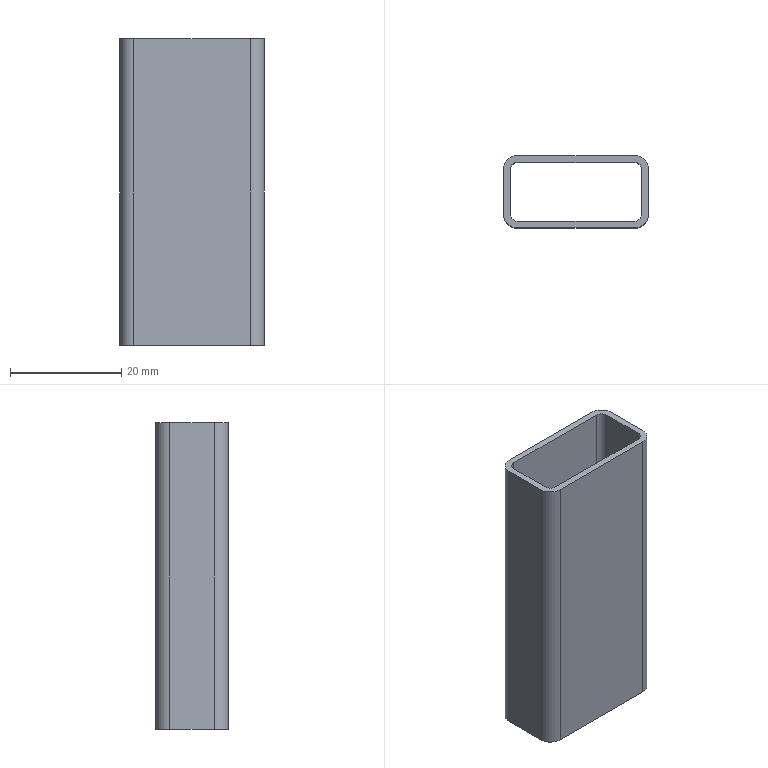Part | STEP file | Q7C0511 | 1 solid | 18 faces | box 26 x 13 x 55 mm | volume 4616 mm3 | plane 10 | cylinder 8 | commonest cylinder face diameters 2.6 x4 5 x4
STEP:
#1=CARTESIAN_POINT('',(0.,0.,0.));
#2=DIRECTION('',(0.,0.,1.));
#3=DIRECTION('',(1.,0.,0.));
#4=AXIS2_PLACEMENT_3D('',#1,#2,#3);
#5=CARTESIAN_POINT('',(13.,4.,27.5));
#6=VERTEX_POINT('',#5);
#7=CARTESIAN_POINT('',(10.5,6.5,27.5));
#8=VERTEX_POINT('',#7);
#9=CARTESIAN_POINT('',(10.5,4.,27.5));
#10=DIRECTION('',(0.,0.,1.));
#11=DIRECTION('',(-1.,0.,0.));
#12=AXIS2_PLACEMENT_3D('',#9,#10,#11);
#13=CIRCLE('',#12,2.5);
#14=CARTESIAN_POINT('',(10.5,4.,27.5));
#15=DIRECTION('',(0.,0.,-1.));
#16=DIRECTION('',(-1.,0.,0.));
#17=AXIS2_PLACEMENT_3D('',#14,#15,#16);
#18=PLANE('',#17);
#19=CARTESIAN_POINT('',(2.5,0.));
#20=CARTESIAN_POINT('',(2.5,-4.33));
#21=CARTESIAN_POINT('',(-1.25,-2.165));
#22=CARTESIAN_POINT('',(-5.,0.));
#23=CARTESIAN_POINT('',(-1.25,2.165));
#24=CARTESIAN_POINT('',(2.5,4.33));
#25=CARTESIAN_POINT('',(2.5,0.));
#26=(BOUNDED_CURVE()B_SPLINE_CURVE(2,(#19,#20,#21,#22,#23,#24,#25),.UNSPECIFIED.,.T.,.F.)B_SPLINE_CURVE_WITH_KNOTS((1,2,2,2,2,1),(-2.094,0.,2.094,4.189,6.283,8.378),.UNSPECIFIED.)CURVE()GEOMETRIC_REPRESENTATION_ITEM()RATIONAL_B_SPLINE_CURVE((1.,0.5,1.,0.5,1.,0.5,1.))REPRESENTATION_ITEM(''));
#27=(GEOMETRIC_REPRESENTATION_CONTEXT(2)PARAMETRIC_REPRESENTATION_CONTEXT()REPRESENTATION_CONTEXT('',''));
#28=DEFINITIONAL_REPRESENTATION('',(#26),#27);
#29=PCURVE('',#18,#28);
#30=CARTESIAN_POINT('',(10.5,4.,27.5));
#31=DIRECTION('',(0.,0.,-1.));
#32=DIRECTION('',(-1.,0.,0.));
#33=AXIS2_PLACEMENT_3D('',#30,#31,#32);
#34=CYLINDRICAL_SURFACE('',#33,2.5);
#35=CARTESIAN_POINT('',(6.283,0.));
#36=DIRECTION('',(-1.,0.));
#37=VECTOR('',#36,1.);
#38=LINE('',#35,#37);
#39=(GEOMETRIC_REPRESENTATION_CONTEXT(2)PARAMETRIC_REPRESENTATION_CONTEXT()REPRESENTATION_CONTEXT('',''));
#40=DEFINITIONAL_REPRESENTATION('',(#38),#39);
#41=PCURVE('',#34,#40);
#42=SURFACE_CURVE('',#13,(#29,#41),.PCURVE_S1.);
#43=EDGE_CURVE('',#6,#8,#42,.T.);
#44=ORIENTED_EDGE('',*,*,#43,.T.);
#45=CARTESIAN_POINT('',(-10.5,6.5,27.5));
#46=VERTEX_POINT('',#45);
#47=CARTESIAN_POINT('',(-10.5,6.5,27.5));
#48=DIRECTION('',(-1.,0.,0.));
#49=VECTOR('',#48,1.);
#50=LINE('',#47,#49);
#51=CARTESIAN_POINT('',(21.,2.5));
#52=DIRECTION('',(1.,0.));
#53=VECTOR('',#52,1.);
#54=LINE('',#51,#53);
#55=(GEOMETRIC_REPRESENTATION_CONTEXT(2)PARAMETRIC_REPRESENTATION_CONTEXT()REPRESENTATION_CONTEXT('',''));
#56=DEFINITIONAL_REPRESENTATION('',(#54),#55);
#57=PCURVE('',#18,#56);
#58=CARTESIAN_POINT('',(-10.5,6.5,27.5));
#59=DIRECTION('',(0.,-1.,0.));
#60=DIRECTION('',(1.,0.,0.));
#61=AXIS2_PLACEMENT_3D('',#58,#59,#60);
#62=PLANE('',#61);
#63=CARTESIAN_POINT('',(0.,0.));
#64=DIRECTION('',(-1.,0.));
#65=VECTOR('',#64,1.);
#66=LINE('',#63,#65);
#67=(GEOMETRIC_REPRESENTATION_CONTEXT(2)PARAMETRIC_REPRESENTATION_CONTEXT()REPRESENTATION_CONTEXT('',''));
#68=DEFINITIONAL_REPRESENTATION('',(#66),#67);
#69=PCURVE('',#62,#68);
#70=SURFACE_CURVE('',#50,(#57,#69),.PCURVE_S1.);
#71=EDGE_CURVE('',#8,#46,#70,.T.);
#72=ORIENTED_EDGE('',*,*,#71,.T.);
#73=CARTESIAN_POINT('',(-13.,4.,27.5));
#74=VERTEX_POINT('',#73);
#75=CARTESIAN_POINT('',(-10.5,4.,27.5));
#76=DIRECTION('',(0.,0.,1.));
#77=DIRECTION('',(1.,0.,0.));
#78=AXIS2_PLACEMENT_3D('',#75,#76,#77);
#79=CIRCLE('',#78,2.5);
#80=CARTESIAN_POINT('',(18.5,0.));
#81=CARTESIAN_POINT('',(18.5,4.33));
#82=CARTESIAN_POINT('',(22.25,2.165));
#83=CARTESIAN_POINT('',(26.,0.));
#84=CARTESIAN_POINT('',(22.25,-2.165));
#85=CARTESIAN_POINT('',(18.5,-4.33));
#86=CARTESIAN_POINT('',(18.5,0.));
#87=(BOUNDED_CURVE()B_SPLINE_CURVE(2,(#80,#81,#82,#83,#84,#85,#86),.UNSPECIFIED.,.T.,.F.)B_SPLINE_CURVE_WITH_KNOTS((1,2,2,2,2,1),(-2.094,0.,2.094,4.189,6.283,8.378),.UNSPECIFIED.)CURVE()GEOMETRIC_REPRESENTATION_ITEM()RATIONAL_B_SPLINE_CURVE((1.,0.5,1.,0.5,1.,0.5,1.))REPRESENTATION_ITEM(''));
#88=(GEOMETRIC_REPRESENTATION_CONTEXT(2)PARAMETRIC_REPRESENTATION_CONTEXT()REPRESENTATION_CONTEXT('',''));
#89=DEFINITIONAL_REPRESENTATION('',(#87),#88);
#90=PCURVE('',#18,#89);
#91=CARTESIAN_POINT('',(-10.5,4.,27.5));
#92=DIRECTION('',(0.,0.,-1.));
#93=DIRECTION('',(-1.,0.,0.));
#94=AXIS2_PLACEMENT_3D('',#91,#92,#93);
#95=CYLINDRICAL_SURFACE('',#94,2.5);
#96=CARTESIAN_POINT('',(3.142,0.));
#97=DIRECTION('',(-1.,0.));
#98=VECTOR('',#97,1.);
#99=LINE('',#96,#98);
#100=(GEOMETRIC_REPRESENTATION_CONTEXT(2)PARAMETRIC_REPRESENTATION_CONTEXT()REPRESENTATION_CONTEXT('',''));
#101=DEFINITIONAL_REPRESENTATION('',(#99),#100);
#102=PCURVE('',#95,#101);
#103=SURFACE_CURVE('',#79,(#90,#102),.PCURVE_S1.);
#104=EDGE_CURVE('',#46,#74,#103,.T.);
#105=ORIENTED_EDGE('',*,*,#104,.T.);
#106=CARTESIAN_POINT('',(-13.,-4.,27.5));
#107=VERTEX_POINT('',#106);
#108=CARTESIAN_POINT('',(-13.,4.,27.5));
#109=DIRECTION('',(0.,-1.,0.));
#110=VECTOR('',#109,1.);
#111=LINE('',#108,#110);
#112=CARTESIAN_POINT('',(23.5,0.));
#113=DIRECTION('',(0.,-1.));
#114=VECTOR('',#113,1.);
#115=LINE('',#112,#114);
#116=(GEOMETRIC_REPRESENTATION_CONTEXT(2)PARAMETRIC_REPRESENTATION_CONTEXT()REPRESENTATION_CONTEXT('',''));
#117=DEFINITIONAL_REPRESENTATION('',(#115),#116);
#118=PCURVE('',#18,#117);
#119=CARTESIAN_POINT('',(-13.,4.,27.5));
#120=DIRECTION('',(1.,0.,0.));
#121=DIRECTION('',(0.,0.,-1.));
#122=AXIS2_PLACEMENT_3D('',#119,#120,#121);
#123=PLANE('',#122);
#124=CARTESIAN_POINT('',(0.,0.));
#125=DIRECTION('',(0.,-1.));
#126=VECTOR('',#125,1.);
#127=LINE('',#124,#126);
#128=(GEOMETRIC_REPRESENTATION_CONTEXT(2)PARAMETRIC_REPRESENTATION_CONTEXT()REPRESENTATION_CONTEXT('',''));
#129=DEFINITIONAL_REPRESENTATION('',(#127),#128);
#130=PCURVE('',#123,#129);
#131=SURFACE_CURVE('',#111,(#118,#130),.PCURVE_S1.);
#132=EDGE_CURVE('',#74,#107,#131,.T.);
#133=ORIENTED_EDGE('',*,*,#132,.T.);
#134=CARTESIAN_POINT('',(-10.5,-6.5,27.5));
#135=VERTEX_POINT('',#134);
#136=CARTESIAN_POINT('',(-10.5,-4.,27.5));
#137=DIRECTION('',(0.,0.,1.));
#138=DIRECTION('',(1.,0.,0.));
#139=AXIS2_PLACEMENT_3D('',#136,#137,#138);
#140=CIRCLE('',#139,2.5);
#141=CARTESIAN_POINT('',(18.5,-8.));
#142=CARTESIAN_POINT('',(18.5,-3.67));
#143=CARTESIAN_POINT('',(22.25,-5.835));
#144=CARTESIAN_POINT('',(26.,-8.));
#145=CARTESIAN_POINT('',(22.25,-10.165));
#146=CARTESIAN_POINT('',(18.5,-12.33));
#147=CARTESIAN_POINT('',(18.5,-8.));
#148=(BOUNDED_CURVE()B_SPLINE_CURVE(2,(#141,#142,#143,#144,#145,#146,#147),.UNSPECIFIED.,.T.,.F.)B_SPLINE_CURVE_WITH_KNOTS((1,2,2,2,2,1),(-2.094,0.,2.094,4.189,6.283,8.378),.UNSPECIFIED.)CURVE()GEOMETRIC_REPRESENTATION_ITEM()RATIONAL_B_SPLINE_CURVE((1.,0.5,1.,0.5,1.,0.5,1.))REPRESENTATION_ITEM(''));
#149=(GEOMETRIC_REPRESENTATION_CONTEXT(2)PARAMETRIC_REPRESENTATION_CONTEXT()REPRESENTATION_CONTEXT('',''));
#150=DEFINITIONAL_REPRESENTATION('',(#148),#149);
#151=PCURVE('',#18,#150);
#152=CARTESIAN_POINT('',(-10.5,-4.,27.5));
#153=DIRECTION('',(0.,0.,-1.));
#154=DIRECTION('',(-1.,0.,0.));
#155=AXIS2_PLACEMENT_3D('',#152,#153,#154);
#156=CYLINDRICAL_SURFACE('',#155,2.5);
#157=CARTESIAN_POINT('',(9.425,0.));
#158=DIRECTION('',(-1.,0.));
#159=VECTOR('',#158,1.);
#160=LINE('',#157,#159);
#161=(GEOMETRIC_REPRESENTATION_CONTEXT(2)PARAMETRIC_REPRESENTATION_CONTEXT()REPRESENTATION_CONTEXT('',''));
#162=DEFINITIONAL_REPRESENTATION('',(#160),#161);
#163=PCURVE('',#156,#162);
#164=SURFACE_CURVE('',#140,(#151,#163),.PCURVE_S1.);
#165=EDGE_CURVE('',#107,#135,#164,.T.);
#166=ORIENTED_EDGE('',*,*,#165,.T.);
#167=CARTESIAN_POINT('',(10.5,-6.5,27.5));
#168=VERTEX_POINT('',#167);
#169=CARTESIAN_POINT('',(-10.5,-6.5,27.5));
#170=DIRECTION('',(1.,0.,0.));
#171=VECTOR('',#170,1.);
#172=LINE('',#169,#171);
#173=CARTESIAN_POINT('',(21.,-10.5));
#174=DIRECTION('',(-1.,0.));
#175=VECTOR('',#174,1.);
#176=LINE('',#173,#175);
#177=(GEOMETRIC_REPRESENTATION_CONTEXT(2)PARAMETRIC_REPRESENTATION_CONTEXT()REPRESENTATION_CONTEXT('',''));
#178=DEFINITIONAL_REPRESENTATION('',(#176),#177);
#179=PCURVE('',#18,#178);
#180=CARTESIAN_POINT('',(-10.5,-6.5,27.5));
#181=DIRECTION('',(0.,1.,0.));
#182=DIRECTION('',(-1.,0.,0.));
#183=AXIS2_PLACEMENT_3D('',#180,#181,#182);
#184=PLANE('',#183);
#185=CARTESIAN_POINT('',(0.,0.));
#186=DIRECTION('',(-1.,0.));
#187=VECTOR('',#186,1.);
#188=LINE('',#185,#187);
#189=(GEOMETRIC_REPRESENTATION_CONTEXT(2)PARAMETRIC_REPRESENTATION_CONTEXT()REPRESENTATION_CONTEXT('',''));
#190=DEFINITIONAL_REPRESENTATION('',(#188),#189);
#191=PCURVE('',#184,#190);
#192=SURFACE_CURVE('',#172,(#179,#191),.PCURVE_S1.);
#193=EDGE_CURVE('',#135,#168,#192,.T.);
#194=ORIENTED_EDGE('',*,*,#193,.T.);
#195=CARTESIAN_POINT('',(13.,-4.,27.5));
#196=VERTEX_POINT('',#195);
#197=CARTESIAN_POINT('',(10.5,-4.,27.5));
#198=DIRECTION('',(0.,0.,1.));
#199=DIRECTION('',(-1.,0.,0.));
#200=AXIS2_PLACEMENT_3D('',#197,#198,#199);
#201=CIRCLE('',#200,2.5);
#202=CARTESIAN_POINT('',(2.5,-8.));
#203=CARTESIAN_POINT('',(2.5,-12.33));
#204=CARTESIAN_POINT('',(-1.25,-10.165));
#205=CARTESIAN_POINT('',(-5.,-8.));
#206=CARTESIAN_POINT('',(-1.25,-5.835));
#207=CARTESIAN_POINT('',(2.5,-3.67));
#208=CARTESIAN_POINT('',(2.5,-8.));
#209=(BOUNDED_CURVE()B_SPLINE_CURVE(2,(#202,#203,#204,#205,#206,#207,#208),.UNSPECIFIED.,.T.,.F.)B_SPLINE_CURVE_WITH_KNOTS((1,2,2,2,2,1),(-2.094,0.,2.094,4.189,6.283,8.378),.UNSPECIFIED.)CURVE()GEOMETRIC_REPRESENTATION_ITEM()RATIONAL_B_SPLINE_CURVE((1.,0.5,1.,0.5,1.,0.5,1.))REPRESENTATION_ITEM(''));
#210=(GEOMETRIC_REPRESENTATION_CONTEXT(2)PARAMETRIC_REPRESENTATION_CONTEXT()REPRESENTATION_CONTEXT('',''));
#211=DEFINITIONAL_REPRESENTATION('',(#209),#210);
#212=PCURVE('',#18,#211);
#213=CARTESIAN_POINT('',(10.5,-4.,27.5));
#214=DIRECTION('',(0.,0.,-1.));
#215=DIRECTION('',(-1.,0.,0.));
#216=AXIS2_PLACEMENT_3D('',#213,#214,#215);
#217=CYLINDRICAL_SURFACE('',#216,2.5);
#218=CARTESIAN_POINT('',(6.283,0.));
#219=DIRECTION('',(-1.,0.));
#220=VECTOR('',#219,1.);
#221=LINE('',#218,#220);
#222=(GEOMETRIC_REPRESENTATION_CONTEXT(2)PARAMETRIC_REPRESENTATION_CONTEXT()REPRESENTATION_CONTEXT('',''));
#223=DEFINITIONAL_REPRESENTATION('',(#221),#222);
#224=PCURVE('',#217,#223);
#225=SURFACE_CURVE('',#201,(#212,#224),.PCURVE_S1.);
#226=EDGE_CURVE('',#168,#196,#225,.T.);
#227=ORIENTED_EDGE('',*,*,#226,.T.);
#228=CARTESIAN_POINT('',(13.,4.,27.5));
#229=DIRECTION('',(0.,1.,0.));
#230=VECTOR('',#229,1.);
#231=LINE('',#228,#230);
#232=CARTESIAN_POINT('',(-2.5,0.));
#233=DIRECTION('',(0.,1.));
#234=VECTOR('',#233,1.);
#235=LINE('',#232,#234);
#236=(GEOMETRIC_REPRESENTATION_CONTEXT(2)PARAMETRIC_REPRESENTATION_CONTEXT()REPRESENTATION_CONTEXT('',''));
#237=DEFINITIONAL_REPRESENTATION('',(#235),#236);
#238=PCURVE('',#18,#237);
#239=CARTESIAN_POINT('',(13.,4.,27.5));
#240=DIRECTION('',(-1.,0.,0.));
#241=DIRECTION('',(0.,-1.,0.));
#242=AXIS2_PLACEMENT_3D('',#239,#240,#241);
#243=PLANE('',#242);
#244=CARTESIAN_POINT('',(0.,0.));
#245=DIRECTION('',(-1.,0.));
#246=VECTOR('',#245,1.);
#247=LINE('',#244,#246);
#248=(GEOMETRIC_REPRESENTATION_CONTEXT(2)PARAMETRIC_REPRESENTATION_CONTEXT()REPRESENTATION_CONTEXT('',''));
#249=DEFINITIONAL_REPRESENTATION('',(#247),#248);
#250=PCURVE('',#243,#249);
#251=SURFACE_CURVE('',#231,(#238,#250),.PCURVE_S1.);
#252=EDGE_CURVE('',#196,#6,#251,.T.);
#253=ORIENTED_EDGE('',*,*,#252,.T.);
#254=EDGE_LOOP('',(#44,#72,#105,#133,#166,#194,#227,#253));
#255=FACE_BOUND('',#254,.T.);
#256=CARTESIAN_POINT('',(-10.5,5.3,27.5));
#257=VERTEX_POINT('',#256);
#258=CARTESIAN_POINT('',(-11.8,4.,27.5));
#259=VERTEX_POINT('',#258);
#260=CARTESIAN_POINT('',(-10.5,4.,27.5));
#261=DIRECTION('',(0.,0.,1.));
#262=DIRECTION('',(1.,0.,0.));
#263=AXIS2_PLACEMENT_3D('',#260,#261,#262);
#264=CIRCLE('',#263,1.3);
#265=CARTESIAN_POINT('',(19.7,0.));
#266=CARTESIAN_POINT('',(19.7,2.252));
#267=CARTESIAN_POINT('',(21.65,1.126));
#268=CARTESIAN_POINT('',(23.6,0.));
#269=CARTESIAN_POINT('',(21.65,-1.126));
#270=CARTESIAN_POINT('',(19.7,-2.252));
#271=CARTESIAN_POINT('',(19.7,0.));
#272=(BOUNDED_CURVE()B_SPLINE_CURVE(2,(#265,#266,#267,#268,#269,#270,#271),.UNSPECIFIED.,.T.,.F.)B_SPLINE_CURVE_WITH_KNOTS((1,2,2,2,2,1),(-2.094,0.,2.094,4.189,6.283,8.378),.UNSPECIFIED.)CURVE()GEOMETRIC_REPRESENTATION_ITEM()RATIONAL_B_SPLINE_CURVE((1.,0.5,1.,0.5,1.,0.5,1.))REPRESENTATION_ITEM(''));
#273=(GEOMETRIC_REPRESENTATION_CONTEXT(2)PARAMETRIC_REPRESENTATION_CONTEXT()REPRESENTATION_CONTEXT('',''));
#274=DEFINITIONAL_REPRESENTATION('',(#272),#273);
#275=PCURVE('',#18,#274);
#276=CARTESIAN_POINT('',(-10.5,4.,27.5));
#277=DIRECTION('',(0.,0.,-1.));
#278=DIRECTION('',(-1.,0.,0.));
#279=AXIS2_PLACEMENT_3D('',#276,#277,#278);
#280=CYLINDRICAL_SURFACE('',#279,1.3);
#281=CARTESIAN_POINT('',(3.142,0.));
#282=DIRECTION('',(-1.,0.));
#283=VECTOR('',#282,1.);
#284=LINE('',#281,#283);
#285=(GEOMETRIC_REPRESENTATION_CONTEXT(2)PARAMETRIC_REPRESENTATION_CONTEXT()REPRESENTATION_CONTEXT('',''));
#286=DEFINITIONAL_REPRESENTATION('',(#284),#285);
#287=PCURVE('',#280,#286);
#288=SURFACE_CURVE('',#264,(#275,#287),.PCURVE_S1.);
#289=EDGE_CURVE('',#257,#259,#288,.T.);
#290=ORIENTED_EDGE('',*,*,#289,.F.);
#291=CARTESIAN_POINT('',(10.5,5.3,27.5));
#292=VERTEX_POINT('',#291);
#293=CARTESIAN_POINT('',(-10.5,5.3,27.5));
#294=DIRECTION('',(-1.,0.,0.));
#295=VECTOR('',#294,1.);
#296=LINE('',#293,#295);
#297=CARTESIAN_POINT('',(21.,1.3));
#298=DIRECTION('',(1.,0.));
#299=VECTOR('',#298,1.);
#300=LINE('',#297,#299);
#301=(GEOMETRIC_REPRESENTATION_CONTEXT(2)PARAMETRIC_REPRESENTATION_CONTEXT()REPRESENTATION_CONTEXT('',''));
#302=DEFINITIONAL_REPRESENTATION('',(#300),#301);
#303=PCURVE('',#18,#302);
#304=CARTESIAN_POINT('',(-10.5,5.3,27.5));
#305=DIRECTION('',(0.,-1.,0.));
#306=DIRECTION('',(0.,0.,-1.));
#307=AXIS2_PLACEMENT_3D('',#304,#305,#306);
#308=PLANE('',#307);
#309=CARTESIAN_POINT('',(0.,0.));
#310=DIRECTION('',(0.,-1.));
#311=VECTOR('',#310,1.);
#312=LINE('',#309,#311);
#313=(GEOMETRIC_REPRESENTATION_CONTEXT(2)PARAMETRIC_REPRESENTATION_CONTEXT()REPRESENTATION_CONTEXT('',''));
#314=DEFINITIONAL_REPRESENTATION('',(#312),#313);
#315=PCURVE('',#308,#314);
#316=SURFACE_CURVE('',#296,(#303,#315),.PCURVE_S1.);
#317=EDGE_CURVE('',#292,#257,#316,.T.);
#318=ORIENTED_EDGE('',*,*,#317,.F.);
#319=CARTESIAN_POINT('',(11.8,4.,27.5));
#320=VERTEX_POINT('',#319);
#321=CARTESIAN_POINT('',(10.5,4.,27.5));
#322=DIRECTION('',(0.,0.,1.));
#323=DIRECTION('',(-1.,0.,0.));
#324=AXIS2_PLACEMENT_3D('',#321,#322,#323);
#325=CIRCLE('',#324,1.3);
#326=CARTESIAN_POINT('',(1.3,0.));
#327=CARTESIAN_POINT('',(1.3,-2.252));
#328=CARTESIAN_POINT('',(-0.65,-1.126));
#329=CARTESIAN_POINT('',(-2.6,0.));
#330=CARTESIAN_POINT('',(-0.65,1.126));
#331=CARTESIAN_POINT('',(1.3,2.252));
#332=CARTESIAN_POINT('',(1.3,0.));
#333=(BOUNDED_CURVE()B_SPLINE_CURVE(2,(#326,#327,#328,#329,#330,#331,#332),.UNSPECIFIED.,.T.,.F.)B_SPLINE_CURVE_WITH_KNOTS((1,2,2,2,2,1),(-2.094,0.,2.094,4.189,6.283,8.378),.UNSPECIFIED.)CURVE()GEOMETRIC_REPRESENTATION_ITEM()RATIONAL_B_SPLINE_CURVE((1.,0.5,1.,0.5,1.,0.5,1.))REPRESENTATION_ITEM(''));
#334=(GEOMETRIC_REPRESENTATION_CONTEXT(2)PARAMETRIC_REPRESENTATION_CONTEXT()REPRESENTATION_CONTEXT('',''));
#335=DEFINITIONAL_REPRESENTATION('',(#333),#334);
#336=PCURVE('',#18,#335);
#337=CARTESIAN_POINT('',(10.5,4.,27.5));
#338=DIRECTION('',(0.,0.,-1.));
#339=DIRECTION('',(-1.,0.,0.));
#340=AXIS2_PLACEMENT_3D('',#337,#338,#339);
#341=CYLINDRICAL_SURFACE('',#340,1.3);
#342=CARTESIAN_POINT('',(6.283,0.));
#343=DIRECTION('',(-1.,0.));
#344=VECTOR('',#343,1.);
#345=LINE('',#342,#344);
#346=(GEOMETRIC_REPRESENTATION_CONTEXT(2)PARAMETRIC_REPRESENTATION_CONTEXT()REPRESENTATION_CONTEXT('',''));
#347=DEFINITIONAL_REPRESENTATION('',(#345),#346);
#348=PCURVE('',#341,#347);
#349=SURFACE_CURVE('',#325,(#336,#348),.PCURVE_S1.);
#350=EDGE_CURVE('',#320,#292,#349,.T.);
#351=ORIENTED_EDGE('',*,*,#350,.F.);
#352=CARTESIAN_POINT('',(11.8,-4.,27.5));
#353=VERTEX_POINT('',#352);
#354=CARTESIAN_POINT('',(11.8,4.,27.5));
#355=DIRECTION('',(0.,1.,0.));
#356=VECTOR('',#355,1.);
#357=LINE('',#354,#356);
#358=CARTESIAN_POINT('',(-1.3,0.));
#359=DIRECTION('',(0.,1.));
#360=VECTOR('',#359,1.);
#361=LINE('',#358,#360);
#362=(GEOMETRIC_REPRESENTATION_CONTEXT(2)PARAMETRIC_REPRESENTATION_CONTEXT()REPRESENTATION_CONTEXT('',''));
#363=DEFINITIONAL_REPRESENTATION('',(#361),#362);
#364=PCURVE('',#18,#363);
#365=CARTESIAN_POINT('',(11.8,4.,27.5));
#366=DIRECTION('',(-1.,0.,0.));
#367=DIRECTION('',(0.,-1.,0.));
#368=AXIS2_PLACEMENT_3D('',#365,#366,#367);
#369=PLANE('',#368);
#370=CARTESIAN_POINT('',(0.,0.));
#371=DIRECTION('',(-1.,0.));
#372=VECTOR('',#371,1.);
#373=LINE('',#370,#372);
#374=(GEOMETRIC_REPRESENTATION_CONTEXT(2)PARAMETRIC_REPRESENTATION_CONTEXT()REPRESENTATION_CONTEXT('',''));
#375=DEFINITIONAL_REPRESENTATION('',(#373),#374);
#376=PCURVE('',#369,#375);
#377=SURFACE_CURVE('',#357,(#364,#376),.PCURVE_S1.);
#378=EDGE_CURVE('',#353,#320,#377,.T.);
#379=ORIENTED_EDGE('',*,*,#378,.F.);
#380=CARTESIAN_POINT('',(10.5,-5.3,27.5));
#381=VERTEX_POINT('',#380);
#382=CARTESIAN_POINT('',(10.5,-4.,27.5));
#383=DIRECTION('',(0.,0.,1.));
#384=DIRECTION('',(-1.,0.,0.));
#385=AXIS2_PLACEMENT_3D('',#382,#383,#384);
#386=CIRCLE('',#385,1.3);
#387=CARTESIAN_POINT('',(1.3,-8.));
#388=CARTESIAN_POINT('',(1.3,-10.252));
#389=CARTESIAN_POINT('',(-0.65,-9.126));
#390=CARTESIAN_POINT('',(-2.6,-8.));
#391=CARTESIAN_POINT('',(-0.65,-6.874));
#392=CARTESIAN_POINT('',(1.3,-5.748));
#393=CARTESIAN_POINT('',(1.3,-8.));
#394=(BOUNDED_CURVE()B_SPLINE_CURVE(2,(#387,#388,#389,#390,#391,#392,#393),.UNSPECIFIED.,.T.,.F.)B_SPLINE_CURVE_WITH_KNOTS((1,2,2,2,2,1),(-2.094,0.,2.094,4.189,6.283,8.378),.UNSPECIFIED.)CURVE()GEOMETRIC_REPRESENTATION_ITEM()RATIONAL_B_SPLINE_CURVE((1.,0.5,1.,0.5,1.,0.5,1.))REPRESENTATION_ITEM(''));
#395=(GEOMETRIC_REPRESENTATION_CONTEXT(2)PARAMETRIC_REPRESENTATION_CONTEXT()REPRESENTATION_CONTEXT('',''));
#396=DEFINITIONAL_REPRESENTATION('',(#394),#395);
#397=PCURVE('',#18,#396);
#398=CARTESIAN_POINT('',(10.5,-4.,27.5));
#399=DIRECTION('',(0.,0.,-1.));
#400=DIRECTION('',(-1.,0.,0.));
#401=AXIS2_PLACEMENT_3D('',#398,#399,#400);
#402=CYLINDRICAL_SURFACE('',#401,1.3);
#403=CARTESIAN_POINT('',(6.283,0.));
#404=DIRECTION('',(-1.,0.));
#405=VECTOR('',#404,1.);
#406=LINE('',#403,#405);
#407=(GEOMETRIC_REPRESENTATION_CONTEXT(2)PARAMETRIC_REPRESENTATION_CONTEXT()REPRESENTATION_CONTEXT('',''));
#408=DEFINITIONAL_REPRESENTATION('',(#406),#407);
#409=PCURVE('',#402,#408);
#410=SURFACE_CURVE('',#386,(#397,#409),.PCURVE_S1.);
#411=EDGE_CURVE('',#381,#353,#410,.T.);
#412=ORIENTED_EDGE('',*,*,#411,.F.);
#413=CARTESIAN_POINT('',(-10.5,-5.3,27.5));
#414=VERTEX_POINT('',#413);
#415=CARTESIAN_POINT('',(-10.5,-5.3,27.5));
#416=DIRECTION('',(1.,0.,0.));
#417=VECTOR('',#416,1.);
#418=LINE('',#415,#417);
#419=CARTESIAN_POINT('',(21.,-9.3));
#420=DIRECTION('',(-1.,0.));
#421=VECTOR('',#420,1.);
#422=LINE('',#419,#421);
#423=(GEOMETRIC_REPRESENTATION_CONTEXT(2)PARAMETRIC_REPRESENTATION_CONTEXT()REPRESENTATION_CONTEXT('',''));
#424=DEFINITIONAL_REPRESENTATION('',(#422),#423);
#425=PCURVE('',#18,#424);
#426=CARTESIAN_POINT('',(-10.5,-5.3,27.5));
#427=DIRECTION('',(0.,1.,0.));
#428=DIRECTION('',(-1.,0.,0.));
#429=AXIS2_PLACEMENT_3D('',#426,#427,#428);
#430=PLANE('',#429);
#431=CARTESIAN_POINT('',(0.,0.));
#432=DIRECTION('',(-1.,0.));
#433=VECTOR('',#432,1.);
#434=LINE('',#431,#433);
#435=(GEOMETRIC_REPRESENTATION_CONTEXT(2)PARAMETRIC_REPRESENTATION_CONTEXT()REPRESENTATION_CONTEXT('',''));
#436=DEFINITIONAL_REPRESENTATION('',(#434),#435);
#437=PCURVE('',#430,#436);
#438=SURFACE_CURVE('',#418,(#425,#437),.PCURVE_S1.);
#439=EDGE_CURVE('',#414,#381,#438,.T.);
#440=ORIENTED_EDGE('',*,*,#439,.F.);
#441=CARTESIAN_POINT('',(-11.8,-4.,27.5));
#442=VERTEX_POINT('',#441);
#443=CARTESIAN_POINT('',(-10.5,-4.,27.5));
#444=DIRECTION('',(0.,0.,1.));
#445=DIRECTION('',(1.,0.,0.));
#446=AXIS2_PLACEMENT_3D('',#443,#444,#445);
#447=CIRCLE('',#446,1.3);
#448=CARTESIAN_POINT('',(19.7,-8.));
#449=CARTESIAN_POINT('',(19.7,-5.748));
#450=CARTESIAN_POINT('',(21.65,-6.874));
#451=CARTESIAN_POINT('',(23.6,-8.));
#452=CARTESIAN_POINT('',(21.65,-9.126));
#453=CARTESIAN_POINT('',(19.7,-10.252));
#454=CARTESIAN_POINT('',(19.7,-8.));
#455=(BOUNDED_CURVE()B_SPLINE_CURVE(2,(#448,#449,#450,#451,#452,#453,#454),.UNSPECIFIED.,.T.,.F.)B_SPLINE_CURVE_WITH_KNOTS((1,2,2,2,2,1),(-2.094,0.,2.094,4.189,6.283,8.378),.UNSPECIFIED.)CURVE()GEOMETRIC_REPRESENTATION_ITEM()RATIONAL_B_SPLINE_CURVE((1.,0.5,1.,0.5,1.,0.5,1.))REPRESENTATION_ITEM(''));
#456=(GEOMETRIC_REPRESENTATION_CONTEXT(2)PARAMETRIC_REPRESENTATION_CONTEXT()REPRESENTATION_CONTEXT('',''));
#457=DEFINITIONAL_REPRESENTATION('',(#455),#456);
#458=PCURVE('',#18,#457);
#459=CARTESIAN_POINT('',(-10.5,-4.,27.5));
#460=DIRECTION('',(0.,0.,-1.));
#461=DIRECTION('',(-1.,0.,0.));
#462=AXIS2_PLACEMENT_3D('',#459,#460,#461);
#463=CYLINDRICAL_SURFACE('',#462,1.3);
#464=CARTESIAN_POINT('',(9.425,0.));
#465=DIRECTION('',(-1.,0.));
#466=VECTOR('',#465,1.);
#467=LINE('',#464,#466);
#468=(GEOMETRIC_REPRESENTATION_CONTEXT(2)PARAMETRIC_REPRESENTATION_CONTEXT()REPRESENTATION_CONTEXT('',''));
#469=DEFINITIONAL_REPRESENTATION('',(#467),#468);
#470=PCURVE('',#463,#469);
#471=SURFACE_CURVE('',#447,(#458,#470),.PCURVE_S1.);
#472=EDGE_CURVE('',#442,#414,#471,.T.);
#473=ORIENTED_EDGE('',*,*,#472,.F.);
#474=CARTESIAN_POINT('',(-11.8,4.,27.5));
#475=DIRECTION('',(0.,-1.,0.));
#476=VECTOR('',#475,1.);
#477=LINE('',#474,#476);
#478=CARTESIAN_POINT('',(22.3,0.));
#479=DIRECTION('',(0.,-1.));
#480=VECTOR('',#479,1.);
#481=LINE('',#478,#480);
#482=(GEOMETRIC_REPRESENTATION_CONTEXT(2)PARAMETRIC_REPRESENTATION_CONTEXT()REPRESENTATION_CONTEXT('',''));
#483=DEFINITIONAL_REPRESENTATION('',(#481),#482);
#484=PCURVE('',#18,#483);
#485=CARTESIAN_POINT('',(-11.8,4.,27.5));
#486=DIRECTION('',(1.,0.,0.));
#487=DIRECTION('',(0.,1.,0.));
#488=AXIS2_PLACEMENT_3D('',#485,#486,#487);
#489=PLANE('',#488);
#490=CARTESIAN_POINT('',(0.,0.));
#491=DIRECTION('',(-1.,0.));
#492=VECTOR('',#491,1.);
#493=LINE('',#490,#492);
#494=(GEOMETRIC_REPRESENTATION_CONTEXT(2)PARAMETRIC_REPRESENTATION_CONTEXT()REPRESENTATION_CONTEXT('',''));
#495=DEFINITIONAL_REPRESENTATION('',(#493),#494);
#496=PCURVE('',#489,#495);
#497=SURFACE_CURVE('',#477,(#484,#496),.PCURVE_S1.);
#498=EDGE_CURVE('',#259,#442,#497,.T.);
#499=ORIENTED_EDGE('',*,*,#498,.F.);
#500=EDGE_LOOP('',(#290,#318,#351,#379,#412,#440,#473,#499));
#501=FACE_BOUND('',#500,.T.);
#502=ADVANCED_FACE('',(#255,#501),#18,.F.);
#503=CARTESIAN_POINT('',(13.,4.,-27.5));
#504=VERTEX_POINT('',#503);
#505=CARTESIAN_POINT('',(10.5,6.5,-27.5));
#506=VERTEX_POINT('',#505);
#507=CARTESIAN_POINT('',(10.5,4.,-27.5));
#508=DIRECTION('',(0.,0.,1.));
#509=DIRECTION('',(-1.,0.,0.));
#510=AXIS2_PLACEMENT_3D('',#507,#508,#509);
#511=CIRCLE('',#510,2.5);
#512=CARTESIAN_POINT('',(10.5,4.,-27.5));
#513=DIRECTION('',(0.,0.,-1.));
#514=DIRECTION('',(-1.,0.,0.));
#515=AXIS2_PLACEMENT_3D('',#512,#513,#514);
#516=PLANE('',#515);
#517=CARTESIAN_POINT('',(2.5,0.));
#518=CARTESIAN_POINT('',(2.5,-4.33));
#519=CARTESIAN_POINT('',(-1.25,-2.165));
#520=CARTESIAN_POINT('',(-5.,0.));
#521=CARTESIAN_POINT('',(-1.25,2.165));
#522=CARTESIAN_POINT('',(2.5,4.33));
#523=CARTESIAN_POINT('',(2.5,0.));
#524=(BOUNDED_CURVE()B_SPLINE_CURVE(2,(#517,#518,#519,#520,#521,#522,#523),.UNSPECIFIED.,.T.,.F.)B_SPLINE_CURVE_WITH_KNOTS((1,2,2,2,2,1),(-2.094,0.,2.094,4.189,6.283,8.378),.UNSPECIFIED.)CURVE()GEOMETRIC_REPRESENTATION_ITEM()RATIONAL_B_SPLINE_CURVE((1.,0.5,1.,0.5,1.,0.5,1.))REPRESENTATION_ITEM(''));
#525=(GEOMETRIC_REPRESENTATION_CONTEXT(2)PARAMETRIC_REPRESENTATION_CONTEXT()REPRESENTATION_CONTEXT('',''));
#526=DEFINITIONAL_REPRESENTATION('',(#524),#525);
#527=PCURVE('',#516,#526);
#528=CARTESIAN_POINT('',(6.283,55.));
#529=DIRECTION('',(-1.,0.));
#530=VECTOR('',#529,1.);
#531=LINE('',#528,#530);
#532=(GEOMETRIC_REPRESENTATION_CONTEXT(2)PARAMETRIC_REPRESENTATION_CONTEXT()REPRESENTATION_CONTEXT('',''));
#533=DEFINITIONAL_REPRESENTATION('',(#531),#532);
#534=PCURVE('',#34,#533);
#535=SURFACE_CURVE('',#511,(#527,#534),.PCURVE_S1.);
#536=EDGE_CURVE('',#504,#506,#535,.T.);
#537=ORIENTED_EDGE('',*,*,#536,.F.);
#538=CARTESIAN_POINT('',(13.,-4.,-27.5));
#539=VERTEX_POINT('',#538);
#540=CARTESIAN_POINT('',(13.,4.,-27.5));
#541=DIRECTION('',(0.,1.,0.));
#542=VECTOR('',#541,1.);
#543=LINE('',#540,#542);
#544=CARTESIAN_POINT('',(-2.5,0.));
#545=DIRECTION('',(0.,1.));
#546=VECTOR('',#545,1.);
#547=LINE('',#544,#546);
#548=(GEOMETRIC_REPRESENTATION_CONTEXT(2)PARAMETRIC_REPRESENTATION_CONTEXT()REPRESENTATION_CONTEXT('',''));
#549=DEFINITIONAL_REPRESENTATION('',(#547),#548);
#550=PCURVE('',#516,#549);
#551=CARTESIAN_POINT('',(0.,-55.));
#552=DIRECTION('',(-1.,0.));
#553=VECTOR('',#552,1.);
#554=LINE('',#551,#553);
#555=(GEOMETRIC_REPRESENTATION_CONTEXT(2)PARAMETRIC_REPRESENTATION_CONTEXT()REPRESENTATION_CONTEXT('',''));
#556=DEFINITIONAL_REPRESENTATION('',(#554),#555);
#557=PCURVE('',#243,#556);
#558=SURFACE_CURVE('',#543,(#550,#557),.PCURVE_S1.);
#559=EDGE_CURVE('',#539,#504,#558,.T.);
#560=ORIENTED_EDGE('',*,*,#559,.F.);
#561=CARTESIAN_POINT('',(10.5,-6.5,-27.5));
#562=VERTEX_POINT('',#561);
#563=CARTESIAN_POINT('',(10.5,-4.,-27.5));
#564=DIRECTION('',(0.,0.,1.));
#565=DIRECTION('',(-1.,0.,0.));
#566=AXIS2_PLACEMENT_3D('',#563,#564,#565);
#567=CIRCLE('',#566,2.5);
#568=CARTESIAN_POINT('',(2.5,-8.));
#569=CARTESIAN_POINT('',(2.5,-12.33));
#570=CARTESIAN_POINT('',(-1.25,-10.165));
#571=CARTESIAN_POINT('',(-5.,-8.));
#572=CARTESIAN_POINT('',(-1.25,-5.835));
#573=CARTESIAN_POINT('',(2.5,-3.67));
#574=CARTESIAN_POINT('',(2.5,-8.));
#575=(BOUNDED_CURVE()B_SPLINE_CURVE(2,(#568,#569,#570,#571,#572,#573,#574),.UNSPECIFIED.,.T.,.F.)B_SPLINE_CURVE_WITH_KNOTS((1,2,2,2,2,1),(-2.094,0.,2.094,4.189,6.283,8.378),.UNSPECIFIED.)CURVE()GEOMETRIC_REPRESENTATION_ITEM()RATIONAL_B_SPLINE_CURVE((1.,0.5,1.,0.5,1.,0.5,1.))REPRESENTATION_ITEM(''));
#576=(GEOMETRIC_REPRESENTATION_CONTEXT(2)PARAMETRIC_REPRESENTATION_CONTEXT()REPRESENTATION_CONTEXT('',''));
#577=DEFINITIONAL_REPRESENTATION('',(#575),#576);
#578=PCURVE('',#516,#577);
#579=CARTESIAN_POINT('',(6.283,55.));
#580=DIRECTION('',(-1.,0.));
#581=VECTOR('',#580,1.);
#582=LINE('',#579,#581);
#583=(GEOMETRIC_REPRESENTATION_CONTEXT(2)PARAMETRIC_REPRESENTATION_CONTEXT()REPRESENTATION_CONTEXT('',''));
#584=DEFINITIONAL_REPRESENTATION('',(#582),#583);
#585=PCURVE('',#217,#584);
#586=SURFACE_CURVE('',#567,(#578,#585),.PCURVE_S1.);
#587=EDGE_CURVE('',#562,#539,#586,.T.);
#588=ORIENTED_EDGE('',*,*,#587,.F.);
#589=CARTESIAN_POINT('',(-10.5,-6.5,-27.5));
#590=VERTEX_POINT('',#589);
#591=CARTESIAN_POINT('',(-10.5,-6.5,-27.5));
#592=DIRECTION('',(1.,0.,0.));
#593=VECTOR('',#592,1.);
#594=LINE('',#591,#593);
#595=CARTESIAN_POINT('',(21.,-10.5));
#596=DIRECTION('',(-1.,0.));
#597=VECTOR('',#596,1.);
#598=LINE('',#595,#597);
#599=(GEOMETRIC_REPRESENTATION_CONTEXT(2)PARAMETRIC_REPRESENTATION_CONTEXT()REPRESENTATION_CONTEXT('',''));
#600=DEFINITIONAL_REPRESENTATION('',(#598),#599);
#601=PCURVE('',#516,#600);
#602=CARTESIAN_POINT('',(0.,-55.));
#603=DIRECTION('',(-1.,0.));
#604=VECTOR('',#603,1.);
#605=LINE('',#602,#604);
#606=(GEOMETRIC_REPRESENTATION_CONTEXT(2)PARAMETRIC_REPRESENTATION_CONTEXT()REPRESENTATION_CONTEXT('',''));
#607=DEFINITIONAL_REPRESENTATION('',(#605),#606);
#608=PCURVE('',#184,#607);
#609=SURFACE_CURVE('',#594,(#601,#608),.PCURVE_S1.);
#610=EDGE_CURVE('',#590,#562,#609,.T.);
#611=ORIENTED_EDGE('',*,*,#610,.F.);
#612=CARTESIAN_POINT('',(-13.,-4.,-27.5));
#613=VERTEX_POINT('',#612);
#614=CARTESIAN_POINT('',(-10.5,-4.,-27.5));
#615=DIRECTION('',(0.,0.,1.));
#616=DIRECTION('',(1.,0.,0.));
#617=AXIS2_PLACEMENT_3D('',#614,#615,#616);
#618=CIRCLE('',#617,2.5);
#619=CARTESIAN_POINT('',(18.5,-8.));
#620=CARTESIAN_POINT('',(18.5,-3.67));
#621=CARTESIAN_POINT('',(22.25,-5.835));
#622=CARTESIAN_POINT('',(26.,-8.));
#623=CARTESIAN_POINT('',(22.25,-10.165));
#624=CARTESIAN_POINT('',(18.5,-12.33));
#625=CARTESIAN_POINT('',(18.5,-8.));
#626=(BOUNDED_CURVE()B_SPLINE_CURVE(2,(#619,#620,#621,#622,#623,#624,#625),.UNSPECIFIED.,.T.,.F.)B_SPLINE_CURVE_WITH_KNOTS((1,2,2,2,2,1),(-2.094,0.,2.094,4.189,6.283,8.378),.UNSPECIFIED.)CURVE()GEOMETRIC_REPRESENTATION_ITEM()RATIONAL_B_SPLINE_CURVE((1.,0.5,1.,0.5,1.,0.5,1.))REPRESENTATION_ITEM(''));
#627=(GEOMETRIC_REPRESENTATION_CONTEXT(2)PARAMETRIC_REPRESENTATION_CONTEXT()REPRESENTATION_CONTEXT('',''));
#628=DEFINITIONAL_REPRESENTATION('',(#626),#627);
#629=PCURVE('',#516,#628);
#630=CARTESIAN_POINT('',(9.425,55.));
#631=DIRECTION('',(-1.,0.));
#632=VECTOR('',#631,1.);
#633=LINE('',#630,#632);
#634=(GEOMETRIC_REPRESENTATION_CONTEXT(2)PARAMETRIC_REPRESENTATION_CONTEXT()REPRESENTATION_CONTEXT('',''));
#635=DEFINITIONAL_REPRESENTATION('',(#633),#634);
#636=PCURVE('',#156,#635);
#637=SURFACE_CURVE('',#618,(#629,#636),.PCURVE_S1.);
#638=EDGE_CURVE('',#613,#590,#637,.T.);
#639=ORIENTED_EDGE('',*,*,#638,.F.);
#640=CARTESIAN_POINT('',(-13.,4.,-27.5));
#641=VERTEX_POINT('',#640);
#642=CARTESIAN_POINT('',(-13.,4.,-27.5));
#643=DIRECTION('',(0.,-1.,0.));
#644=VECTOR('',#643,1.);
#645=LINE('',#642,#644);
#646=CARTESIAN_POINT('',(23.5,0.));
#647=DIRECTION('',(0.,-1.));
#648=VECTOR('',#647,1.);
#649=LINE('',#646,#648);
#650=(GEOMETRIC_REPRESENTATION_CONTEXT(2)PARAMETRIC_REPRESENTATION_CONTEXT()REPRESENTATION_CONTEXT('',''));
#651=DEFINITIONAL_REPRESENTATION('',(#649),#650);
#652=PCURVE('',#516,#651);
#653=CARTESIAN_POINT('',(55.,0.));
#654=DIRECTION('',(0.,-1.));
#655=VECTOR('',#654,1.);
#656=LINE('',#653,#655);
#657=(GEOMETRIC_REPRESENTATION_CONTEXT(2)PARAMETRIC_REPRESENTATION_CONTEXT()REPRESENTATION_CONTEXT('',''));
#658=DEFINITIONAL_REPRESENTATION('',(#656),#657);
#659=PCURVE('',#123,#658);
#660=SURFACE_CURVE('',#645,(#652,#659),.PCURVE_S1.);
#661=EDGE_CURVE('',#641,#613,#660,.T.);
#662=ORIENTED_EDGE('',*,*,#661,.F.);
#663=CARTESIAN_POINT('',(-10.5,6.5,-27.5));
#664=VERTEX_POINT('',#663);
#665=CARTESIAN_POINT('',(-10.5,4.,-27.5));
#666=DIRECTION('',(0.,0.,1.));
#667=DIRECTION('',(1.,0.,0.));
#668=AXIS2_PLACEMENT_3D('',#665,#666,#667);
#669=CIRCLE('',#668,2.5);
#670=CARTESIAN_POINT('',(18.5,0.));
#671=CARTESIAN_POINT('',(18.5,4.33));
#672=CARTESIAN_POINT('',(22.25,2.165));
#673=CARTESIAN_POINT('',(26.,0.));
#674=CARTESIAN_POINT('',(22.25,-2.165));
#675=CARTESIAN_POINT('',(18.5,-4.33));
#676=CARTESIAN_POINT('',(18.5,0.));
#677=(BOUNDED_CURVE()B_SPLINE_CURVE(2,(#670,#671,#672,#673,#674,#675,#676),.UNSPECIFIED.,.T.,.F.)B_SPLINE_CURVE_WITH_KNOTS((1,2,2,2,2,1),(-2.094,0.,2.094,4.189,6.283,8.378),.UNSPECIFIED.)CURVE()GEOMETRIC_REPRESENTATION_ITEM()RATIONAL_B_SPLINE_CURVE((1.,0.5,1.,0.5,1.,0.5,1.))REPRESENTATION_ITEM(''));
#678=(GEOMETRIC_REPRESENTATION_CONTEXT(2)PARAMETRIC_REPRESENTATION_CONTEXT()REPRESENTATION_CONTEXT('',''));
#679=DEFINITIONAL_REPRESENTATION('',(#677),#678);
#680=PCURVE('',#516,#679);
#681=CARTESIAN_POINT('',(3.142,55.));
#682=DIRECTION('',(-1.,0.));
#683=VECTOR('',#682,1.);
#684=LINE('',#681,#683);
#685=(GEOMETRIC_REPRESENTATION_CONTEXT(2)PARAMETRIC_REPRESENTATION_CONTEXT()REPRESENTATION_CONTEXT('',''));
#686=DEFINITIONAL_REPRESENTATION('',(#684),#685);
#687=PCURVE('',#95,#686);
#688=SURFACE_CURVE('',#669,(#680,#687),.PCURVE_S1.);
#689=EDGE_CURVE('',#664,#641,#688,.T.);
#690=ORIENTED_EDGE('',*,*,#689,.F.);
#691=CARTESIAN_POINT('',(-10.5,6.5,-27.5));
#692=DIRECTION('',(-1.,0.,0.));
#693=VECTOR('',#692,1.);
#694=LINE('',#691,#693);
#695=CARTESIAN_POINT('',(21.,2.5));
#696=DIRECTION('',(1.,0.));
#697=VECTOR('',#696,1.);
#698=LINE('',#695,#697);
#699=(GEOMETRIC_REPRESENTATION_CONTEXT(2)PARAMETRIC_REPRESENTATION_CONTEXT()REPRESENTATION_CONTEXT('',''));
#700=DEFINITIONAL_REPRESENTATION('',(#698),#699);
#701=PCURVE('',#516,#700);
#702=CARTESIAN_POINT('',(0.,-55.));
#703=DIRECTION('',(-1.,0.));
#704=VECTOR('',#703,1.);
#705=LINE('',#702,#704);
#706=(GEOMETRIC_REPRESENTATION_CONTEXT(2)PARAMETRIC_REPRESENTATION_CONTEXT()REPRESENTATION_CONTEXT('',''));
#707=DEFINITIONAL_REPRESENTATION('',(#705),#706);
#708=PCURVE('',#62,#707);
#709=SURFACE_CURVE('',#694,(#701,#708),.PCURVE_S1.);
#710=EDGE_CURVE('',#506,#664,#709,.T.);
#711=ORIENTED_EDGE('',*,*,#710,.F.);
#712=EDGE_LOOP('',(#537,#560,#588,#611,#639,#662,#690,#711));
#713=FACE_BOUND('',#712,.T.);
#714=CARTESIAN_POINT('',(10.5,5.3,-27.5));
#715=VERTEX_POINT('',#714);
#716=CARTESIAN_POINT('',(-10.5,5.3,-27.5));
#717=VERTEX_POINT('',#716);
#718=CARTESIAN_POINT('',(-10.5,5.3,-27.5));
#719=DIRECTION('',(-1.,0.,0.));
#720=VECTOR('',#719,1.);
#721=LINE('',#718,#720);
#722=CARTESIAN_POINT('',(21.,1.3));
#723=DIRECTION('',(1.,0.));
#724=VECTOR('',#723,1.);
#725=LINE('',#722,#724);
#726=(GEOMETRIC_REPRESENTATION_CONTEXT(2)PARAMETRIC_REPRESENTATION_CONTEXT()REPRESENTATION_CONTEXT('',''));
#727=DEFINITIONAL_REPRESENTATION('',(#725),#726);
#728=PCURVE('',#516,#727);
#729=CARTESIAN_POINT('',(55.,0.));
#730=DIRECTION('',(0.,-1.));
#731=VECTOR('',#730,1.);
#732=LINE('',#729,#731);
#733=(GEOMETRIC_REPRESENTATION_CONTEXT(2)PARAMETRIC_REPRESENTATION_CONTEXT()REPRESENTATION_CONTEXT('',''));
#734=DEFINITIONAL_REPRESENTATION('',(#732),#733);
#735=PCURVE('',#308,#734);
#736=SURFACE_CURVE('',#721,(#728,#735),.PCURVE_S1.);
#737=EDGE_CURVE('',#715,#717,#736,.T.);
#738=ORIENTED_EDGE('',*,*,#737,.T.);
#739=CARTESIAN_POINT('',(-11.8,4.,-27.5));
#740=VERTEX_POINT('',#739);
#741=CARTESIAN_POINT('',(-10.5,4.,-27.5));
#742=DIRECTION('',(0.,0.,1.));
#743=DIRECTION('',(1.,0.,0.));
#744=AXIS2_PLACEMENT_3D('',#741,#742,#743);
#745=CIRCLE('',#744,1.3);
#746=CARTESIAN_POINT('',(19.7,0.));
#747=CARTESIAN_POINT('',(19.7,2.252));
#748=CARTESIAN_POINT('',(21.65,1.126));
#749=CARTESIAN_POINT('',(23.6,0.));
#750=CARTESIAN_POINT('',(21.65,-1.126));
#751=CARTESIAN_POINT('',(19.7,-2.252));
#752=CARTESIAN_POINT('',(19.7,0.));
#753=(BOUNDED_CURVE()B_SPLINE_CURVE(2,(#746,#747,#748,#749,#750,#751,#752),.UNSPECIFIED.,.T.,.F.)B_SPLINE_CURVE_WITH_KNOTS((1,2,2,2,2,1),(-2.094,0.,2.094,4.189,6.283,8.378),.UNSPECIFIED.)CURVE()GEOMETRIC_REPRESENTATION_ITEM()RATIONAL_B_SPLINE_CURVE((1.,0.5,1.,0.5,1.,0.5,1.))REPRESENTATION_ITEM(''));
#754=(GEOMETRIC_REPRESENTATION_CONTEXT(2)PARAMETRIC_REPRESENTATION_CONTEXT()REPRESENTATION_CONTEXT('',''));
#755=DEFINITIONAL_REPRESENTATION('',(#753),#754);
#756=PCURVE('',#516,#755);
#757=CARTESIAN_POINT('',(3.142,55.));
#758=DIRECTION('',(-1.,0.));
#759=VECTOR('',#758,1.);
#760=LINE('',#757,#759);
#761=(GEOMETRIC_REPRESENTATION_CONTEXT(2)PARAMETRIC_REPRESENTATION_CONTEXT()REPRESENTATION_CONTEXT('',''));
#762=DEFINITIONAL_REPRESENTATION('',(#760),#761);
#763=PCURVE('',#280,#762);
#764=SURFACE_CURVE('',#745,(#756,#763),.PCURVE_S1.);
#765=EDGE_CURVE('',#717,#740,#764,.T.);
#766=ORIENTED_EDGE('',*,*,#765,.T.);
#767=CARTESIAN_POINT('',(-11.8,-4.,-27.5));
#768=VERTEX_POINT('',#767);
#769=CARTESIAN_POINT('',(-11.8,4.,-27.5));
#770=DIRECTION('',(0.,-1.,0.));
#771=VECTOR('',#770,1.);
#772=LINE('',#769,#771);
#773=CARTESIAN_POINT('',(22.3,0.));
#774=DIRECTION('',(0.,-1.));
#775=VECTOR('',#774,1.);
#776=LINE('',#773,#775);
#777=(GEOMETRIC_REPRESENTATION_CONTEXT(2)PARAMETRIC_REPRESENTATION_CONTEXT()REPRESENTATION_CONTEXT('',''));
#778=DEFINITIONAL_REPRESENTATION('',(#776),#777);
#779=PCURVE('',#516,#778);
#780=CARTESIAN_POINT('',(0.,-55.));
#781=DIRECTION('',(-1.,0.));
#782=VECTOR('',#781,1.);
#783=LINE('',#780,#782);
#784=(GEOMETRIC_REPRESENTATION_CONTEXT(2)PARAMETRIC_REPRESENTATION_CONTEXT()REPRESENTATION_CONTEXT('',''));
#785=DEFINITIONAL_REPRESENTATION('',(#783),#784);
#786=PCURVE('',#489,#785);
#787=SURFACE_CURVE('',#772,(#779,#786),.PCURVE_S1.);
#788=EDGE_CURVE('',#740,#768,#787,.T.);
#789=ORIENTED_EDGE('',*,*,#788,.T.);
#790=CARTESIAN_POINT('',(-10.5,-5.3,-27.5));
#791=VERTEX_POINT('',#790);
#792=CARTESIAN_POINT('',(-10.5,-4.,-27.5));
#793=DIRECTION('',(0.,0.,1.));
#794=DIRECTION('',(1.,0.,0.));
#795=AXIS2_PLACEMENT_3D('',#792,#793,#794);
#796=CIRCLE('',#795,1.3);
#797=CARTESIAN_POINT('',(19.7,-8.));
#798=CARTESIAN_POINT('',(19.7,-5.748));
#799=CARTESIAN_POINT('',(21.65,-6.874));
#800=CARTESIAN_POINT('',(23.6,-8.));
#801=CARTESIAN_POINT('',(21.65,-9.126));
#802=CARTESIAN_POINT('',(19.7,-10.252));
#803=CARTESIAN_POINT('',(19.7,-8.));
#804=(BOUNDED_CURVE()B_SPLINE_CURVE(2,(#797,#798,#799,#800,#801,#802,#803),.UNSPECIFIED.,.T.,.F.)B_SPLINE_CURVE_WITH_KNOTS((1,2,2,2,2,1),(-2.094,0.,2.094,4.189,6.283,8.378),.UNSPECIFIED.)CURVE()GEOMETRIC_REPRESENTATION_ITEM()RATIONAL_B_SPLINE_CURVE((1.,0.5,1.,0.5,1.,0.5,1.))REPRESENTATION_ITEM(''));
#805=(GEOMETRIC_REPRESENTATION_CONTEXT(2)PARAMETRIC_REPRESENTATION_CONTEXT()REPRESENTATION_CONTEXT('',''));
#806=DEFINITIONAL_REPRESENTATION('',(#804),#805);
#807=PCURVE('',#516,#806);
#808=CARTESIAN_POINT('',(9.425,55.));
#809=DIRECTION('',(-1.,0.));
#810=VECTOR('',#809,1.);
#811=LINE('',#808,#810);
#812=(GEOMETRIC_REPRESENTATION_CONTEXT(2)PARAMETRIC_REPRESENTATION_CONTEXT()REPRESENTATION_CONTEXT('',''));
#813=DEFINITIONAL_REPRESENTATION('',(#811),#812);
#814=PCURVE('',#463,#813);
#815=SURFACE_CURVE('',#796,(#807,#814),.PCURVE_S1.);
#816=EDGE_CURVE('',#768,#791,#815,.T.);
#817=ORIENTED_EDGE('',*,*,#816,.T.);
#818=CARTESIAN_POINT('',(10.5,-5.3,-27.5));
#819=VERTEX_POINT('',#818);
#820=CARTESIAN_POINT('',(-10.5,-5.3,-27.5));
#821=DIRECTION('',(1.,0.,0.));
#822=VECTOR('',#821,1.);
#823=LINE('',#820,#822);
#824=CARTESIAN_POINT('',(21.,-9.3));
#825=DIRECTION('',(-1.,0.));
#826=VECTOR('',#825,1.);
#827=LINE('',#824,#826);
#828=(GEOMETRIC_REPRESENTATION_CONTEXT(2)PARAMETRIC_REPRESENTATION_CONTEXT()REPRESENTATION_CONTEXT('',''));
#829=DEFINITIONAL_REPRESENTATION('',(#827),#828);
#830=PCURVE('',#516,#829);
#831=CARTESIAN_POINT('',(0.,-55.));
#832=DIRECTION('',(-1.,0.));
#833=VECTOR('',#832,1.);
#834=LINE('',#831,#833);
#835=(GEOMETRIC_REPRESENTATION_CONTEXT(2)PARAMETRIC_REPRESENTATION_CONTEXT()REPRESENTATION_CONTEXT('',''));
#836=DEFINITIONAL_REPRESENTATION('',(#834),#835);
#837=PCURVE('',#430,#836);
#838=SURFACE_CURVE('',#823,(#830,#837),.PCURVE_S1.);
#839=EDGE_CURVE('',#791,#819,#838,.T.);
#840=ORIENTED_EDGE('',*,*,#839,.T.);
#841=CARTESIAN_POINT('',(11.8,-4.,-27.5));
#842=VERTEX_POINT('',#841);
#843=CARTESIAN_POINT('',(10.5,-4.,-27.5));
#844=DIRECTION('',(0.,0.,1.));
#845=DIRECTION('',(-1.,0.,0.));
#846=AXIS2_PLACEMENT_3D('',#843,#844,#845);
#847=CIRCLE('',#846,1.3);
#848=CARTESIAN_POINT('',(1.3,-8.));
#849=CARTESIAN_POINT('',(1.3,-10.252));
#850=CARTESIAN_POINT('',(-0.65,-9.126));
#851=CARTESIAN_POINT('',(-2.6,-8.));
#852=CARTESIAN_POINT('',(-0.65,-6.874));
#853=CARTESIAN_POINT('',(1.3,-5.748));
#854=CARTESIAN_POINT('',(1.3,-8.));
#855=(BOUNDED_CURVE()B_SPLINE_CURVE(2,(#848,#849,#850,#851,#852,#853,#854),.UNSPECIFIED.,.T.,.F.)B_SPLINE_CURVE_WITH_KNOTS((1,2,2,2,2,1),(-2.094,0.,2.094,4.189,6.283,8.378),.UNSPECIFIED.)CURVE()GEOMETRIC_REPRESENTATION_ITEM()RATIONAL_B_SPLINE_CURVE((1.,0.5,1.,0.5,1.,0.5,1.))REPRESENTATION_ITEM(''));
#856=(GEOMETRIC_REPRESENTATION_CONTEXT(2)PARAMETRIC_REPRESENTATION_CONTEXT()REPRESENTATION_CONTEXT('',''));
#857=DEFINITIONAL_REPRESENTATION('',(#855),#856);
#858=PCURVE('',#516,#857);
#859=CARTESIAN_POINT('',(6.283,55.));
#860=DIRECTION('',(-1.,0.));
#861=VECTOR('',#860,1.);
#862=LINE('',#859,#861);
#863=(GEOMETRIC_REPRESENTATION_CONTEXT(2)PARAMETRIC_REPRESENTATION_CONTEXT()REPRESENTATION_CONTEXT('',''));
#864=DEFINITIONAL_REPRESENTATION('',(#862),#863);
#865=PCURVE('',#402,#864);
#866=SURFACE_CURVE('',#847,(#858,#865),.PCURVE_S1.);
#867=EDGE_CURVE('',#819,#842,#866,.T.);
#868=ORIENTED_EDGE('',*,*,#867,.T.);
#869=CARTESIAN_POINT('',(11.8,4.,-27.5));
#870=VERTEX_POINT('',#869);
#871=CARTESIAN_POINT('',(11.8,4.,-27.5));
#872=DIRECTION('',(0.,1.,0.));
#873=VECTOR('',#872,1.);
#874=LINE('',#871,#873);
#875=CARTESIAN_POINT('',(-1.3,0.));
#876=DIRECTION('',(0.,1.));
#877=VECTOR('',#876,1.);
#878=LINE('',#875,#877);
#879=(GEOMETRIC_REPRESENTATION_CONTEXT(2)PARAMETRIC_REPRESENTATION_CONTEXT()REPRESENTATION_CONTEXT('',''));
#880=DEFINITIONAL_REPRESENTATION('',(#878),#879);
#881=PCURVE('',#516,#880);
#882=CARTESIAN_POINT('',(0.,-55.));
#883=DIRECTION('',(-1.,0.));
#884=VECTOR('',#883,1.);
#885=LINE('',#882,#884);
#886=(GEOMETRIC_REPRESENTATION_CONTEXT(2)PARAMETRIC_REPRESENTATION_CONTEXT()REPRESENTATION_CONTEXT('',''));
#887=DEFINITIONAL_REPRESENTATION('',(#885),#886);
#888=PCURVE('',#369,#887);
#889=SURFACE_CURVE('',#874,(#881,#888),.PCURVE_S1.);
#890=EDGE_CURVE('',#842,#870,#889,.T.);
#891=ORIENTED_EDGE('',*,*,#890,.T.);
#892=CARTESIAN_POINT('',(10.5,4.,-27.5));
#893=DIRECTION('',(0.,0.,1.));
#894=DIRECTION('',(-1.,0.,0.));
#895=AXIS2_PLACEMENT_3D('',#892,#893,#894);
#896=CIRCLE('',#895,1.3);
#897=CARTESIAN_POINT('',(1.3,0.));
#898=CARTESIAN_POINT('',(1.3,-2.252));
#899=CARTESIAN_POINT('',(-0.65,-1.126));
#900=CARTESIAN_POINT('',(-2.6,0.));
#901=CARTESIAN_POINT('',(-0.65,1.126));
#902=CARTESIAN_POINT('',(1.3,2.252));
#903=CARTESIAN_POINT('',(1.3,0.));
#904=(BOUNDED_CURVE()B_SPLINE_CURVE(2,(#897,#898,#899,#900,#901,#902,#903),.UNSPECIFIED.,.T.,.F.)B_SPLINE_CURVE_WITH_KNOTS((1,2,2,2,2,1),(-2.094,0.,2.094,4.189,6.283,8.378),.UNSPECIFIED.)CURVE()GEOMETRIC_REPRESENTATION_ITEM()RATIONAL_B_SPLINE_CURVE((1.,0.5,1.,0.5,1.,0.5,1.))REPRESENTATION_ITEM(''));
#905=(GEOMETRIC_REPRESENTATION_CONTEXT(2)PARAMETRIC_REPRESENTATION_CONTEXT()REPRESENTATION_CONTEXT('',''));
#906=DEFINITIONAL_REPRESENTATION('',(#904),#905);
#907=PCURVE('',#516,#906);
#908=CARTESIAN_POINT('',(6.283,55.));
#909=DIRECTION('',(-1.,0.));
#910=VECTOR('',#909,1.);
#911=LINE('',#908,#910);
#912=(GEOMETRIC_REPRESENTATION_CONTEXT(2)PARAMETRIC_REPRESENTATION_CONTEXT()REPRESENTATION_CONTEXT('',''));
#913=DEFINITIONAL_REPRESENTATION('',(#911),#912);
#914=PCURVE('',#341,#913);
#915=SURFACE_CURVE('',#896,(#907,#914),.PCURVE_S1.);
#916=EDGE_CURVE('',#870,#715,#915,.T.);
#917=ORIENTED_EDGE('',*,*,#916,.T.);
#918=EDGE_LOOP('',(#738,#766,#789,#817,#840,#868,#891,#917));
#919=FACE_BOUND('',#918,.T.);
#920=ADVANCED_FACE('',(#713,#919),#516,.T.);
#921=ORIENTED_EDGE('',*,*,#536,.T.);
#922=CARTESIAN_POINT('',(10.5,6.5,27.5));
#923=DIRECTION('',(0.,0.,-1.));
#924=VECTOR('',#923,1.);
#925=LINE('',#922,#924);
#926=CARTESIAN_POINT('',(1.571,0.));
#927=DIRECTION('',(0.,1.));
#928=VECTOR('',#927,1.);
#929=LINE('',#926,#928);
#930=(GEOMETRIC_REPRESENTATION_CONTEXT(2)PARAMETRIC_REPRESENTATION_CONTEXT()REPRESENTATION_CONTEXT('',''));
#931=DEFINITIONAL_REPRESENTATION('',(#929),#930);
#932=PCURVE('',#34,#931);
#933=CARTESIAN_POINT('',(21.,0.));
#934=DIRECTION('',(0.,-1.));
#935=VECTOR('',#934,1.);
#936=LINE('',#933,#935);
#937=(GEOMETRIC_REPRESENTATION_CONTEXT(2)PARAMETRIC_REPRESENTATION_CONTEXT()REPRESENTATION_CONTEXT('',''));
#938=DEFINITIONAL_REPRESENTATION('',(#936),#937);
#939=PCURVE('',#62,#938);
#940=SURFACE_CURVE('',#925,(#932,#939),.PCURVE_S1.);
#941=EDGE_CURVE('',#8,#506,#940,.T.);
#942=ORIENTED_EDGE('',*,*,#941,.F.);
#943=ORIENTED_EDGE('',*,*,#43,.F.);
#944=CARTESIAN_POINT('',(13.,4.,27.5));
#945=DIRECTION('',(0.,0.,-1.));
#946=VECTOR('',#945,1.);
#947=LINE('',#944,#946);
#948=CARTESIAN_POINT('',(3.142,0.));
#949=DIRECTION('',(0.,1.));
#950=VECTOR('',#949,1.);
#951=LINE('',#948,#950);
#952=(GEOMETRIC_REPRESENTATION_CONTEXT(2)PARAMETRIC_REPRESENTATION_CONTEXT()REPRESENTATION_CONTEXT('',''));
#953=DEFINITIONAL_REPRESENTATION('',(#951),#952);
#954=PCURVE('',#34,#953);
#955=CARTESIAN_POINT('',(0.,0.));
#956=DIRECTION('',(0.,-1.));
#957=VECTOR('',#956,1.);
#958=LINE('',#955,#957);
#959=(GEOMETRIC_REPRESENTATION_CONTEXT(2)PARAMETRIC_REPRESENTATION_CONTEXT()REPRESENTATION_CONTEXT('',''));
#960=DEFINITIONAL_REPRESENTATION('',(#958),#959);
#961=PCURVE('',#243,#960);
#962=SURFACE_CURVE('',#947,(#954,#961),.PCURVE_S1.);
#963=EDGE_CURVE('',#6,#504,#962,.T.);
#964=ORIENTED_EDGE('',*,*,#963,.T.);
#965=EDGE_LOOP('',(#921,#942,#943,#964));
#966=FACE_BOUND('',#965,.T.);
#967=ADVANCED_FACE('',(#966),#34,.T.);
#968=ORIENTED_EDGE('',*,*,#710,.T.);
#969=CARTESIAN_POINT('',(-10.5,6.5,27.5));
#970=DIRECTION('',(0.,0.,-1.));
#971=VECTOR('',#970,1.);
#972=LINE('',#969,#971);
#973=CARTESIAN_POINT('',(0.,0.));
#974=DIRECTION('',(0.,-1.));
#975=VECTOR('',#974,1.);
#976=LINE('',#973,#975);
#977=(GEOMETRIC_REPRESENTATION_CONTEXT(2)PARAMETRIC_REPRESENTATION_CONTEXT()REPRESENTATION_CONTEXT('',''));
#978=DEFINITIONAL_REPRESENTATION('',(#976),#977);
#979=PCURVE('',#62,#978);
#980=CARTESIAN_POINT('',(1.571,0.));
#981=DIRECTION('',(0.,1.));
#982=VECTOR('',#981,1.);
#983=LINE('',#980,#982);
#984=(GEOMETRIC_REPRESENTATION_CONTEXT(2)PARAMETRIC_REPRESENTATION_CONTEXT()REPRESENTATION_CONTEXT('',''));
#985=DEFINITIONAL_REPRESENTATION('',(#983),#984);
#986=PCURVE('',#95,#985);
#987=SURFACE_CURVE('',#972,(#979,#986),.PCURVE_S1.);
#988=EDGE_CURVE('',#46,#664,#987,.T.);
#989=ORIENTED_EDGE('',*,*,#988,.F.);
#990=ORIENTED_EDGE('',*,*,#71,.F.);
#991=ORIENTED_EDGE('',*,*,#941,.T.);
#992=EDGE_LOOP('',(#968,#989,#990,#991));
#993=FACE_BOUND('',#992,.T.);
#994=ADVANCED_FACE('',(#993),#62,.F.);
#995=ORIENTED_EDGE('',*,*,#689,.T.);
#996=CARTESIAN_POINT('',(-13.,4.,27.5));
#997=DIRECTION('',(0.,0.,-1.));
#998=VECTOR('',#997,1.);
#999=LINE('',#996,#998);
#1000=CARTESIAN_POINT('',(0.,0.));
#1001=DIRECTION('',(0.,1.));
#1002=VECTOR('',#1001,1.);
#1003=LINE('',#1000,#1002);
#1004=(GEOMETRIC_REPRESENTATION_CONTEXT(2)PARAMETRIC_REPRESENTATION_CONTEXT()REPRESENTATION_CONTEXT('',''));
#1005=DEFINITIONAL_REPRESENTATION('',(#1003),#1004);
#1006=PCURVE('',#95,#1005);
#1007=CARTESIAN_POINT('',(0.,0.));
#1008=DIRECTION('',(1.,0.));
#1009=VECTOR('',#1008,1.);
#1010=LINE('',#1007,#1009);
#1011=(GEOMETRIC_REPRESENTATION_CONTEXT(2)PARAMETRIC_REPRESENTATION_CONTEXT()REPRESENTATION_CONTEXT('',''));
#1012=DEFINITIONAL_REPRESENTATION('',(#1010),#1011);
#1013=PCURVE('',#123,#1012);
#1014=SURFACE_CURVE('',#999,(#1006,#1013),.PCURVE_S1.);
#1015=EDGE_CURVE('',#74,#641,#1014,.T.);
#1016=ORIENTED_EDGE('',*,*,#1015,.F.);
#1017=ORIENTED_EDGE('',*,*,#104,.F.);
#1018=ORIENTED_EDGE('',*,*,#988,.T.);
#1019=EDGE_LOOP('',(#995,#1016,#1017,#1018));
#1020=FACE_BOUND('',#1019,.T.);
#1021=ADVANCED_FACE('',(#1020),#95,.T.);
#1022=ORIENTED_EDGE('',*,*,#661,.T.);
#1023=CARTESIAN_POINT('',(-13.,-4.,27.5));
#1024=DIRECTION('',(0.,0.,-1.));
#1025=VECTOR('',#1024,1.);
#1026=LINE('',#1023,#1025);
#1027=CARTESIAN_POINT('',(0.,-8.));
#1028=DIRECTION('',(1.,0.));
#1029=VECTOR('',#1028,1.);
#1030=LINE('',#1027,#1029);
#1031=(GEOMETRIC_REPRESENTATION_CONTEXT(2)PARAMETRIC_REPRESENTATION_CONTEXT()REPRESENTATION_CONTEXT('',''));
#1032=DEFINITIONAL_REPRESENTATION('',(#1030),#1031);
#1033=PCURVE('',#123,#1032);
#1034=CARTESIAN_POINT('',(6.283,0.));
#1035=DIRECTION('',(0.,1.));
#1036=VECTOR('',#1035,1.);
#1037=LINE('',#1034,#1036);
#1038=(GEOMETRIC_REPRESENTATION_CONTEXT(2)PARAMETRIC_REPRESENTATION_CONTEXT()REPRESENTATION_CONTEXT('',''));
#1039=DEFINITIONAL_REPRESENTATION('',(#1037),#1038);
#1040=PCURVE('',#156,#1039);
#1041=SURFACE_CURVE('',#1026,(#1033,#1040),.PCURVE_S1.);
#1042=EDGE_CURVE('',#107,#613,#1041,.T.);
#1043=ORIENTED_EDGE('',*,*,#1042,.F.);
#1044=ORIENTED_EDGE('',*,*,#132,.F.);
#1045=ORIENTED_EDGE('',*,*,#1015,.T.);
#1046=EDGE_LOOP('',(#1022,#1043,#1044,#1045));
#1047=FACE_BOUND('',#1046,.T.);
#1048=ADVANCED_FACE('',(#1047),#123,.F.);
#1049=ORIENTED_EDGE('',*,*,#638,.T.);
#1050=CARTESIAN_POINT('',(-10.5,-6.5,27.5));
#1051=DIRECTION('',(0.,0.,-1.));
#1052=VECTOR('',#1051,1.);
#1053=LINE('',#1050,#1052);
#1054=CARTESIAN_POINT('',(4.712,0.));
#1055=DIRECTION('',(0.,1.));
#1056=VECTOR('',#1055,1.);
#1057=LINE('',#1054,#1056);
#1058=(GEOMETRIC_REPRESENTATION_CONTEXT(2)PARAMETRIC_REPRESENTATION_CONTEXT()REPRESENTATION_CONTEXT('',''));
#1059=DEFINITIONAL_REPRESENTATION('',(#1057),#1058);
#1060=PCURVE('',#156,#1059);
#1061=CARTESIAN_POINT('',(0.,0.));
#1062=DIRECTION('',(0.,-1.));
#1063=VECTOR('',#1062,1.);
#1064=LINE('',#1061,#1063);
#1065=(GEOMETRIC_REPRESENTATION_CONTEXT(2)PARAMETRIC_REPRESENTATION_CONTEXT()REPRESENTATION_CONTEXT('',''));
#1066=DEFINITIONAL_REPRESENTATION('',(#1064),#1065);
#1067=PCURVE('',#184,#1066);
#1068=SURFACE_CURVE('',#1053,(#1060,#1067),.PCURVE_S1.);
#1069=EDGE_CURVE('',#135,#590,#1068,.T.);
#1070=ORIENTED_EDGE('',*,*,#1069,.F.);
#1071=ORIENTED_EDGE('',*,*,#165,.F.);
#1072=ORIENTED_EDGE('',*,*,#1042,.T.);
#1073=EDGE_LOOP('',(#1049,#1070,#1071,#1072));
#1074=FACE_BOUND('',#1073,.T.);
#1075=ADVANCED_FACE('',(#1074),#156,.T.);
#1076=ORIENTED_EDGE('',*,*,#610,.T.);
#1077=CARTESIAN_POINT('',(10.5,-6.5,27.5));
#1078=DIRECTION('',(0.,0.,-1.));
#1079=VECTOR('',#1078,1.);
#1080=LINE('',#1077,#1079);
#1081=CARTESIAN_POINT('',(-21.,0.));
#1082=DIRECTION('',(0.,-1.));
#1083=VECTOR('',#1082,1.);
#1084=LINE('',#1081,#1083);
#1085=(GEOMETRIC_REPRESENTATION_CONTEXT(2)PARAMETRIC_REPRESENTATION_CONTEXT()REPRESENTATION_CONTEXT('',''));
#1086=DEFINITIONAL_REPRESENTATION('',(#1084),#1085);
#1087=PCURVE('',#184,#1086);
#1088=CARTESIAN_POINT('',(4.712,0.));
#1089=DIRECTION('',(0.,1.));
#1090=VECTOR('',#1089,1.);
#1091=LINE('',#1088,#1090);
#1092=(GEOMETRIC_REPRESENTATION_CONTEXT(2)PARAMETRIC_REPRESENTATION_CONTEXT()REPRESENTATION_CONTEXT('',''));
#1093=DEFINITIONAL_REPRESENTATION('',(#1091),#1092);
#1094=PCURVE('',#217,#1093);
#1095=SURFACE_CURVE('',#1080,(#1087,#1094),.PCURVE_S1.);
#1096=EDGE_CURVE('',#168,#562,#1095,.T.);
#1097=ORIENTED_EDGE('',*,*,#1096,.F.);
#1098=ORIENTED_EDGE('',*,*,#193,.F.);
#1099=ORIENTED_EDGE('',*,*,#1069,.T.);
#1100=EDGE_LOOP('',(#1076,#1097,#1098,#1099));
#1101=FACE_BOUND('',#1100,.T.);
#1102=ADVANCED_FACE('',(#1101),#184,.F.);
#1103=ORIENTED_EDGE('',*,*,#587,.T.);
#1104=CARTESIAN_POINT('',(13.,-4.,27.5));
#1105=DIRECTION('',(0.,0.,-1.));
#1106=VECTOR('',#1105,1.);
#1107=LINE('',#1104,#1106);
#1108=CARTESIAN_POINT('',(3.142,0.));
#1109=DIRECTION('',(0.,1.));
#1110=VECTOR('',#1109,1.);
#1111=LINE('',#1108,#1110);
#1112=(GEOMETRIC_REPRESENTATION_CONTEXT(2)PARAMETRIC_REPRESENTATION_CONTEXT()REPRESENTATION_CONTEXT('',''));
#1113=DEFINITIONAL_REPRESENTATION('',(#1111),#1112);
#1114=PCURVE('',#217,#1113);
#1115=CARTESIAN_POINT('',(8.,0.));
#1116=DIRECTION('',(0.,-1.));
#1117=VECTOR('',#1116,1.);
#1118=LINE('',#1115,#1117);
#1119=(GEOMETRIC_REPRESENTATION_CONTEXT(2)PARAMETRIC_REPRESENTATION_CONTEXT()REPRESENTATION_CONTEXT('',''));
#1120=DEFINITIONAL_REPRESENTATION('',(#1118),#1119);
#1121=PCURVE('',#243,#1120);
#1122=SURFACE_CURVE('',#1107,(#1114,#1121),.PCURVE_S1.);
#1123=EDGE_CURVE('',#196,#539,#1122,.T.);
#1124=ORIENTED_EDGE('',*,*,#1123,.F.);
#1125=ORIENTED_EDGE('',*,*,#226,.F.);
#1126=ORIENTED_EDGE('',*,*,#1096,.T.);
#1127=EDGE_LOOP('',(#1103,#1124,#1125,#1126));
#1128=FACE_BOUND('',#1127,.T.);
#1129=ADVANCED_FACE('',(#1128),#217,.T.);
#1130=ORIENTED_EDGE('',*,*,#559,.T.);
#1131=ORIENTED_EDGE('',*,*,#963,.F.);
#1132=ORIENTED_EDGE('',*,*,#252,.F.);
#1133=ORIENTED_EDGE('',*,*,#1123,.T.);
#1134=EDGE_LOOP('',(#1130,#1131,#1132,#1133));
#1135=FACE_BOUND('',#1134,.T.);
#1136=ADVANCED_FACE('',(#1135),#243,.F.);
#1137=CARTESIAN_POINT('',(-11.8,4.,27.5));
#1138=DIRECTION('',(0.,0.,-1.));
#1139=VECTOR('',#1138,1.);
#1140=LINE('',#1137,#1139);
#1141=CARTESIAN_POINT('',(0.,0.));
#1142=DIRECTION('',(0.,1.));
#1143=VECTOR('',#1142,1.);
#1144=LINE('',#1141,#1143);
#1145=(GEOMETRIC_REPRESENTATION_CONTEXT(2)PARAMETRIC_REPRESENTATION_CONTEXT()REPRESENTATION_CONTEXT('',''));
#1146=DEFINITIONAL_REPRESENTATION('',(#1144),#1145);
#1147=PCURVE('',#280,#1146);
#1148=CARTESIAN_POINT('',(0.,0.));
#1149=DIRECTION('',(0.,-1.));
#1150=VECTOR('',#1149,1.);
#1151=LINE('',#1148,#1150);
#1152=(GEOMETRIC_REPRESENTATION_CONTEXT(2)PARAMETRIC_REPRESENTATION_CONTEXT()REPRESENTATION_CONTEXT('',''));
#1153=DEFINITIONAL_REPRESENTATION('',(#1151),#1152);
#1154=PCURVE('',#489,#1153);
#1155=SURFACE_CURVE('',#1140,(#1147,#1154),.PCURVE_S1.);
#1156=EDGE_CURVE('',#259,#740,#1155,.T.);
#1157=ORIENTED_EDGE('',*,*,#1156,.F.);
#1158=ORIENTED_EDGE('',*,*,#289,.F.);
#1159=CARTESIAN_POINT('',(-10.5,5.3,27.5));
#1160=DIRECTION('',(0.,0.,-1.));
#1161=VECTOR('',#1160,1.);
#1162=LINE('',#1159,#1161);
#1163=CARTESIAN_POINT('',(1.571,0.));
#1164=DIRECTION('',(0.,1.));
#1165=VECTOR('',#1164,1.);
#1166=LINE('',#1163,#1165);
#1167=(GEOMETRIC_REPRESENTATION_CONTEXT(2)PARAMETRIC_REPRESENTATION_CONTEXT()REPRESENTATION_CONTEXT('',''));
#1168=DEFINITIONAL_REPRESENTATION('',(#1166),#1167);
#1169=PCURVE('',#280,#1168);
#1170=CARTESIAN_POINT('',(0.,0.));
#1171=DIRECTION('',(1.,0.));
#1172=VECTOR('',#1171,1.);
#1173=LINE('',#1170,#1172);
#1174=(GEOMETRIC_REPRESENTATION_CONTEXT(2)PARAMETRIC_REPRESENTATION_CONTEXT()REPRESENTATION_CONTEXT('',''));
#1175=DEFINITIONAL_REPRESENTATION('',(#1173),#1174);
#1176=PCURVE('',#308,#1175);
#1177=SURFACE_CURVE('',#1162,(#1169,#1176),.PCURVE_S1.);
#1178=EDGE_CURVE('',#257,#717,#1177,.T.);
#1179=ORIENTED_EDGE('',*,*,#1178,.T.);
#1180=ORIENTED_EDGE('',*,*,#765,.T.);
#1181=EDGE_LOOP('',(#1157,#1158,#1179,#1180));
#1182=FACE_BOUND('',#1181,.F.);
#1183=ADVANCED_FACE('',(#1182),#280,.F.);
#1184=ORIENTED_EDGE('',*,*,#788,.F.);
#1185=ORIENTED_EDGE('',*,*,#1156,.F.);
#1186=ORIENTED_EDGE('',*,*,#498,.T.);
#1187=CARTESIAN_POINT('',(-11.8,-4.,27.5));
#1188=DIRECTION('',(0.,0.,-1.));
#1189=VECTOR('',#1188,1.);
#1190=LINE('',#1187,#1189);
#1191=CARTESIAN_POINT('',(-8.,0.));
#1192=DIRECTION('',(0.,-1.));
#1193=VECTOR('',#1192,1.);
#1194=LINE('',#1191,#1193);
#1195=(GEOMETRIC_REPRESENTATION_CONTEXT(2)PARAMETRIC_REPRESENTATION_CONTEXT()REPRESENTATION_CONTEXT('',''));
#1196=DEFINITIONAL_REPRESENTATION('',(#1194),#1195);
#1197=PCURVE('',#489,#1196);
#1198=CARTESIAN_POINT('',(6.283,0.));
#1199=DIRECTION('',(0.,1.));
#1200=VECTOR('',#1199,1.);
#1201=LINE('',#1198,#1200);
#1202=(GEOMETRIC_REPRESENTATION_CONTEXT(2)PARAMETRIC_REPRESENTATION_CONTEXT()REPRESENTATION_CONTEXT('',''));
#1203=DEFINITIONAL_REPRESENTATION('',(#1201),#1202);
#1204=PCURVE('',#463,#1203);
#1205=SURFACE_CURVE('',#1190,(#1197,#1204),.PCURVE_S1.);
#1206=EDGE_CURVE('',#442,#768,#1205,.T.);
#1207=ORIENTED_EDGE('',*,*,#1206,.T.);
#1208=EDGE_LOOP('',(#1184,#1185,#1186,#1207));
#1209=FACE_BOUND('',#1208,.T.);
#1210=ADVANCED_FACE('',(#1209),#489,.T.);
#1211=CARTESIAN_POINT('',(-10.5,-5.3,27.5));
#1212=DIRECTION('',(0.,0.,-1.));
#1213=VECTOR('',#1212,1.);
#1214=LINE('',#1211,#1213);
#1215=CARTESIAN_POINT('',(4.712,0.));
#1216=DIRECTION('',(0.,1.));
#1217=VECTOR('',#1216,1.);
#1218=LINE('',#1215,#1217);
#1219=(GEOMETRIC_REPRESENTATION_CONTEXT(2)PARAMETRIC_REPRESENTATION_CONTEXT()REPRESENTATION_CONTEXT('',''));
#1220=DEFINITIONAL_REPRESENTATION('',(#1218),#1219);
#1221=PCURVE('',#463,#1220);
#1222=CARTESIAN_POINT('',(0.,0.));
#1223=DIRECTION('',(0.,-1.));
#1224=VECTOR('',#1223,1.);
#1225=LINE('',#1222,#1224);
#1226=(GEOMETRIC_REPRESENTATION_CONTEXT(2)PARAMETRIC_REPRESENTATION_CONTEXT()REPRESENTATION_CONTEXT('',''));
#1227=DEFINITIONAL_REPRESENTATION('',(#1225),#1226);
#1228=PCURVE('',#430,#1227);
#1229=SURFACE_CURVE('',#1214,(#1221,#1228),.PCURVE_S1.);
#1230=EDGE_CURVE('',#414,#791,#1229,.T.);
#1231=ORIENTED_EDGE('',*,*,#1230,.F.);
#1232=ORIENTED_EDGE('',*,*,#472,.F.);
#1233=ORIENTED_EDGE('',*,*,#1206,.T.);
#1234=ORIENTED_EDGE('',*,*,#816,.T.);
#1235=EDGE_LOOP('',(#1231,#1232,#1233,#1234));
#1236=FACE_BOUND('',#1235,.F.);
#1237=ADVANCED_FACE('',(#1236),#463,.F.);
#1238=ORIENTED_EDGE('',*,*,#839,.F.);
#1239=ORIENTED_EDGE('',*,*,#1230,.F.);
#1240=ORIENTED_EDGE('',*,*,#439,.T.);
#1241=CARTESIAN_POINT('',(10.5,-5.3,27.5));
#1242=DIRECTION('',(0.,0.,-1.));
#1243=VECTOR('',#1242,1.);
#1244=LINE('',#1241,#1243);
#1245=CARTESIAN_POINT('',(-21.,0.));
#1246=DIRECTION('',(0.,-1.));
#1247=VECTOR('',#1246,1.);
#1248=LINE('',#1245,#1247);
#1249=(GEOMETRIC_REPRESENTATION_CONTEXT(2)PARAMETRIC_REPRESENTATION_CONTEXT()REPRESENTATION_CONTEXT('',''));
#1250=DEFINITIONAL_REPRESENTATION('',(#1248),#1249);
#1251=PCURVE('',#430,#1250);
#1252=CARTESIAN_POINT('',(4.712,0.));
#1253=DIRECTION('',(0.,1.));
#1254=VECTOR('',#1253,1.);
#1255=LINE('',#1252,#1254);
#1256=(GEOMETRIC_REPRESENTATION_CONTEXT(2)PARAMETRIC_REPRESENTATION_CONTEXT()REPRESENTATION_CONTEXT('',''));
#1257=DEFINITIONAL_REPRESENTATION('',(#1255),#1256);
#1258=PCURVE('',#402,#1257);
#1259=SURFACE_CURVE('',#1244,(#1251,#1258),.PCURVE_S1.);
#1260=EDGE_CURVE('',#381,#819,#1259,.T.);
#1261=ORIENTED_EDGE('',*,*,#1260,.T.);
#1262=EDGE_LOOP('',(#1238,#1239,#1240,#1261));
#1263=FACE_BOUND('',#1262,.T.);
#1264=ADVANCED_FACE('',(#1263),#430,.T.);
#1265=CARTESIAN_POINT('',(11.8,-4.,27.5));
#1266=DIRECTION('',(0.,0.,-1.));
#1267=VECTOR('',#1266,1.);
#1268=LINE('',#1265,#1267);
#1269=CARTESIAN_POINT('',(3.142,0.));
#1270=DIRECTION('',(0.,1.));
#1271=VECTOR('',#1270,1.);
#1272=LINE('',#1269,#1271);
#1273=(GEOMETRIC_REPRESENTATION_CONTEXT(2)PARAMETRIC_REPRESENTATION_CONTEXT()REPRESENTATION_CONTEXT('',''));
#1274=DEFINITIONAL_REPRESENTATION('',(#1272),#1273);
#1275=PCURVE('',#402,#1274);
#1276=CARTESIAN_POINT('',(8.,0.));
#1277=DIRECTION('',(0.,-1.));
#1278=VECTOR('',#1277,1.);
#1279=LINE('',#1276,#1278);
#1280=(GEOMETRIC_REPRESENTATION_CONTEXT(2)PARAMETRIC_REPRESENTATION_CONTEXT()REPRESENTATION_CONTEXT('',''));
#1281=DEFINITIONAL_REPRESENTATION('',(#1279),#1280);
#1282=PCURVE('',#369,#1281);
#1283=SURFACE_CURVE('',#1268,(#1275,#1282),.PCURVE_S1.);
#1284=EDGE_CURVE('',#353,#842,#1283,.T.);
#1285=ORIENTED_EDGE('',*,*,#1284,.F.);
#1286=ORIENTED_EDGE('',*,*,#411,.F.);
#1287=ORIENTED_EDGE('',*,*,#1260,.T.);
#1288=ORIENTED_EDGE('',*,*,#867,.T.);
#1289=EDGE_LOOP('',(#1285,#1286,#1287,#1288));
#1290=FACE_BOUND('',#1289,.F.);
#1291=ADVANCED_FACE('',(#1290),#402,.F.);
#1292=ORIENTED_EDGE('',*,*,#890,.F.);
#1293=ORIENTED_EDGE('',*,*,#1284,.F.);
#1294=ORIENTED_EDGE('',*,*,#378,.T.);
#1295=CARTESIAN_POINT('',(11.8,4.,27.5));
#1296=DIRECTION('',(0.,0.,-1.));
#1297=VECTOR('',#1296,1.);
#1298=LINE('',#1295,#1297);
#1299=CARTESIAN_POINT('',(0.,0.));
#1300=DIRECTION('',(0.,-1.));
#1301=VECTOR('',#1300,1.);
#1302=LINE('',#1299,#1301);
#1303=(GEOMETRIC_REPRESENTATION_CONTEXT(2)PARAMETRIC_REPRESENTATION_CONTEXT()REPRESENTATION_CONTEXT('',''));
#1304=DEFINITIONAL_REPRESENTATION('',(#1302),#1303);
#1305=PCURVE('',#369,#1304);
#1306=CARTESIAN_POINT('',(3.142,0.));
#1307=DIRECTION('',(0.,1.));
#1308=VECTOR('',#1307,1.);
#1309=LINE('',#1306,#1308);
#1310=(GEOMETRIC_REPRESENTATION_CONTEXT(2)PARAMETRIC_REPRESENTATION_CONTEXT()REPRESENTATION_CONTEXT('',''));
#1311=DEFINITIONAL_REPRESENTATION('',(#1309),#1310);
#1312=PCURVE('',#341,#1311);
#1313=SURFACE_CURVE('',#1298,(#1305,#1312),.PCURVE_S1.);
#1314=EDGE_CURVE('',#320,#870,#1313,.T.);
#1315=ORIENTED_EDGE('',*,*,#1314,.T.);
#1316=EDGE_LOOP('',(#1292,#1293,#1294,#1315));
#1317=FACE_BOUND('',#1316,.T.);
#1318=ADVANCED_FACE('',(#1317),#369,.T.);
#1319=CARTESIAN_POINT('',(10.5,5.3,27.5));
#1320=DIRECTION('',(0.,0.,-1.));
#1321=VECTOR('',#1320,1.);
#1322=LINE('',#1319,#1321);
#1323=CARTESIAN_POINT('',(1.571,0.));
#1324=DIRECTION('',(0.,1.));
#1325=VECTOR('',#1324,1.);
#1326=LINE('',#1323,#1325);
#1327=(GEOMETRIC_REPRESENTATION_CONTEXT(2)PARAMETRIC_REPRESENTATION_CONTEXT()REPRESENTATION_CONTEXT('',''));
#1328=DEFINITIONAL_REPRESENTATION('',(#1326),#1327);
#1329=PCURVE('',#341,#1328);
#1330=CARTESIAN_POINT('',(0.,21.));
#1331=DIRECTION('',(1.,0.));
#1332=VECTOR('',#1331,1.);
#1333=LINE('',#1330,#1332);
#1334=(GEOMETRIC_REPRESENTATION_CONTEXT(2)PARAMETRIC_REPRESENTATION_CONTEXT()REPRESENTATION_CONTEXT('',''));
#1335=DEFINITIONAL_REPRESENTATION('',(#1333),#1334);
#1336=PCURVE('',#308,#1335);
#1337=SURFACE_CURVE('',#1322,(#1329,#1336),.PCURVE_S1.);
#1338=EDGE_CURVE('',#292,#715,#1337,.T.);
#1339=ORIENTED_EDGE('',*,*,#1338,.F.);
#1340=ORIENTED_EDGE('',*,*,#350,.F.);
#1341=ORIENTED_EDGE('',*,*,#1314,.T.);
#1342=ORIENTED_EDGE('',*,*,#916,.T.);
#1343=EDGE_LOOP('',(#1339,#1340,#1341,#1342));
#1344=FACE_BOUND('',#1343,.F.);
#1345=ADVANCED_FACE('',(#1344),#341,.F.);
#1346=ORIENTED_EDGE('',*,*,#737,.F.);
#1347=ORIENTED_EDGE('',*,*,#1338,.F.);
#1348=ORIENTED_EDGE('',*,*,#317,.T.);
#1349=ORIENTED_EDGE('',*,*,#1178,.T.);
#1350=EDGE_LOOP('',(#1346,#1347,#1348,#1349));
#1351=FACE_BOUND('',#1350,.T.);
#1352=ADVANCED_FACE('',(#1351),#308,.T.);
#1353=CLOSED_SHELL('',(#502,#920,#967,#994,#1021,#1048,#1075,#1102,#1129,#1136,#1183,#1210,#1237,#1264,#1291,#1318,#1345,#1352));
#1354=MANIFOLD_SOLID_BREP('',#1353);
#1355=(LENGTH_UNIT()NAMED_UNIT(*)SI_UNIT(.MILLI.,.METRE.));
#1356=UNCERTAINTY_MEASURE_WITH_UNIT(LENGTH_MEASURE(0.0000001),#1355,'','');
#1357=(NAMED_UNIT(*)PLANE_ANGLE_UNIT()SI_UNIT($,.RADIAN.));
#1358=(NAMED_UNIT(*)SI_UNIT($,.STERADIAN.)SOLID_ANGLE_UNIT());
#1359=(GEOMETRIC_REPRESENTATION_CONTEXT(3)GLOBAL_UNCERTAINTY_ASSIGNED_CONTEXT((#1356))GLOBAL_UNIT_ASSIGNED_CONTEXT((#1355,#1357,#1358))REPRESENTATION_CONTEXT('',''));
#1360=ADVANCED_BREP_SHAPE_REPRESENTATION('',(#4,#1354),#1359);